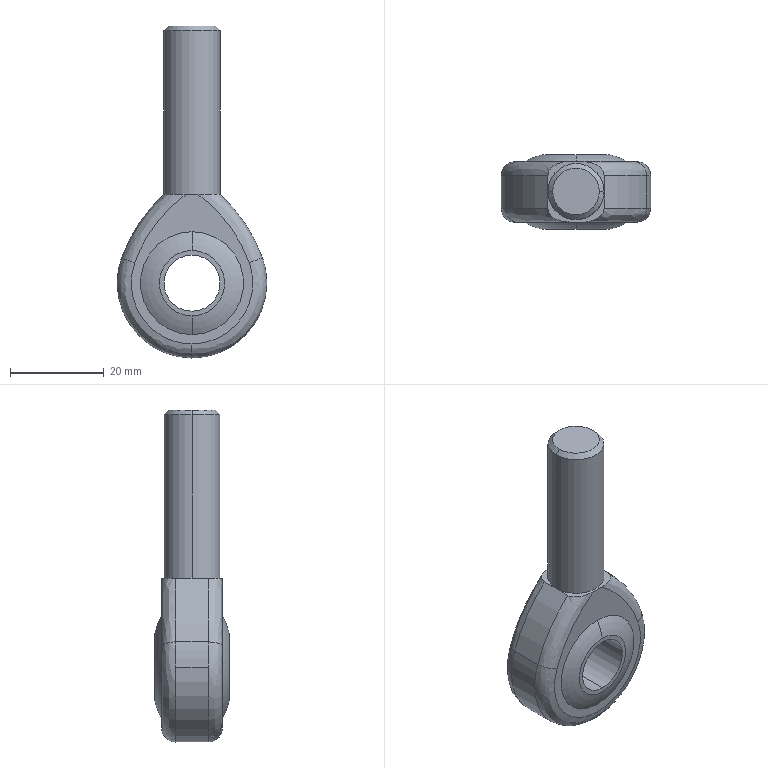Part | SolidWorks | features BaseBody 1 | 1 solid | 30 faces | box 32 x 16 x 71 mm | volume 14151 mm3 | cylinder 9 | spline 8 | plane 7 | torus 4 | cone 2 | commonest cylinder face diameters 12 x4 32 x3 67.817 x2
STEP:
#1=CARTESIAN_POINT('',(5.,0.,36.));
#2=VERTEX_POINT('',#1);
#3=CARTESIAN_POINT('',(-5.,0.,36.));
#4=VERTEX_POINT('',#3);
#5=CARTESIAN_POINT('',(0.,0.,36.));
#6=DIRECTION('',(0.,0.,1.));
#7=DIRECTION('',(-1.,0.,0.));
#8=AXIS2_PLACEMENT_3D('',#5,#6,#7);
#9=CIRCLE('',#8,5.);
#10=EDGE_CURVE('',#2,#4,#9,.T.);
#11=ORIENTED_EDGE('',*,*,#10,.F.);
#12=CARTESIAN_POINT('',(6.,0.,35.));
#13=VERTEX_POINT('',#12);
#14=CARTESIAN_POINT('',(5.,0.,36.));
#15=DIRECTION('',(0.7071,0.,-0.7071));
#16=VECTOR('',#15,1000.);
#17=LINE('',#14,#16);
#18=EDGE_CURVE('',#2,#13,#17,.T.);
#19=ORIENTED_EDGE('',*,*,#18,.T.);
#20=CARTESIAN_POINT('',(-6.,0.,35.));
#21=VERTEX_POINT('',#20);
#22=CARTESIAN_POINT('',(0.,0.,35.));
#23=DIRECTION('',(0.,0.,-1.));
#24=DIRECTION('',(-1.,0.,0.));
#25=AXIS2_PLACEMENT_3D('',#22,#23,#24);
#26=CIRCLE('',#25,6.);
#27=EDGE_CURVE('',#21,#13,#26,.T.);
#28=ORIENTED_EDGE('',*,*,#27,.F.);
#29=CARTESIAN_POINT('',(-5.,0.,36.));
#30=DIRECTION('',(-0.7071,0.,-0.7071));
#31=VECTOR('',#30,1000.);
#32=LINE('',#29,#31);
#33=EDGE_CURVE('',#4,#21,#32,.T.);
#34=ORIENTED_EDGE('',*,*,#33,.F.);
#35=EDGE_LOOP('',(#11,#19,#28,#34));
#36=FACE_OUTER_BOUND('',#35,.T.);
#37=CARTESIAN_POINT('',(0.,0.,36.));
#38=DIRECTION('',(0.,0.,-1.));
#39=DIRECTION('',(-1.,0.,0.));
#40=AXIS2_PLACEMENT_3D('',#37,#38,#39);
#41=CONICAL_SURFACE('',#40,5.,0.7854);
#42=ADVANCED_FACE('',(#36),#41,.T.);
#43=ORIENTED_EDGE('',*,*,#27,.T.);
#44=CARTESIAN_POINT('',(6.,0.,0.));
#45=VERTEX_POINT('',#44);
#46=CARTESIAN_POINT('',(6.,0.,35.));
#47=DIRECTION('',(0.,0.,-1.));
#48=VECTOR('',#47,1000.);
#49=LINE('',#46,#48);
#50=EDGE_CURVE('',#13,#45,#49,.T.);
#51=ORIENTED_EDGE('',*,*,#50,.T.);
#52=CARTESIAN_POINT('',(-6.,-0.000000001,0.));
#53=VERTEX_POINT('',#52);
#54=CARTESIAN_POINT('',(0.,0.,0.));
#55=DIRECTION('',(0.,0.,-1.));
#56=DIRECTION('',(-1.,0.,0.));
#57=AXIS2_PLACEMENT_3D('',#54,#55,#56);
#58=CIRCLE('',#57,6.);
#59=EDGE_CURVE('',#53,#45,#58,.T.);
#60=ORIENTED_EDGE('',*,*,#59,.F.);
#61=CARTESIAN_POINT('',(-6.,0.,35.));
#62=DIRECTION('',(0.,0.,-1.));
#63=VECTOR('',#62,1000.);
#64=LINE('',#61,#63);
#65=EDGE_CURVE('',#21,#53,#64,.T.);
#66=ORIENTED_EDGE('',*,*,#65,.F.);
#67=EDGE_LOOP('',(#43,#51,#60,#66));
#68=FACE_OUTER_BOUND('',#67,.T.);
#69=CARTESIAN_POINT('',(0.,0.,35.));
#70=DIRECTION('',(0.,0.,-1.));
#71=DIRECTION('',(-1.,0.,0.));
#72=AXIS2_PLACEMENT_3D('',#69,#70,#71);
#73=CYLINDRICAL_SURFACE('',#72,6.);
#74=ADVANCED_FACE('',(#68),#73,.T.);
#75=CARTESIAN_POINT('',(-16.,3.5,-19.));
#76=VERTEX_POINT('',#75);
#77=CARTESIAN_POINT('',(-15.06,3.5,-13.597));
#78=VERTEX_POINT('',#77);
#79=CARTESIAN_POINT('',(0.,3.5,-19.));
#80=DIRECTION('',(0.,1.,0.));
#81=DIRECTION('',(1.,0.,0.));
#82=AXIS2_PLACEMENT_3D('',#79,#80,#81);
#83=CIRCLE('',#82,16.);
#84=EDGE_CURVE('',#76,#78,#83,.T.);
#85=ORIENTED_EDGE('',*,*,#84,.F.);
#86=CARTESIAN_POINT('',(-16.,-3.5,-19.));
#87=VERTEX_POINT('',#86);
#88=CARTESIAN_POINT('',(-16.,3.5,-19.));
#89=DIRECTION('',(0.,-1.,0.));
#90=VECTOR('',#89,1000.);
#91=LINE('',#88,#90);
#92=EDGE_CURVE('',#76,#87,#91,.T.);
#93=ORIENTED_EDGE('',*,*,#92,.T.);
#94=CARTESIAN_POINT('',(-15.06,-3.5,-13.597));
#95=VERTEX_POINT('',#94);
#96=CARTESIAN_POINT('',(0.,-3.5,-19.));
#97=DIRECTION('',(0.,-1.,0.));
#98=DIRECTION('',(0.,0.,-1.));
#99=AXIS2_PLACEMENT_3D('',#96,#97,#98);
#100=CIRCLE('',#99,16.);
#101=EDGE_CURVE('',#95,#87,#100,.T.);
#102=ORIENTED_EDGE('',*,*,#101,.F.);
#103=CARTESIAN_POINT('',(-15.06,0.,-13.597));
#104=DIRECTION('',(0.,1.,0.));
#105=VECTOR('',#104,1000.);
#106=LINE('',#103,#105);
#107=EDGE_CURVE('',#95,#78,#106,.T.);
#108=ORIENTED_EDGE('',*,*,#107,.T.);
#109=EDGE_LOOP('',(#85,#93,#102,#108));
#110=FACE_OUTER_BOUND('',#109,.T.);
#111=CARTESIAN_POINT('',(0.,3.5,-19.));
#112=DIRECTION('',(0.,-1.,0.));
#113=DIRECTION('',(1.,0.,0.));
#114=AXIS2_PLACEMENT_3D('',#111,#112,#113);
#115=CYLINDRICAL_SURFACE('',#114,16.);
#116=ADVANCED_FACE('',(#110),#115,.T.);
#117=ORIENTED_EDGE('',*,*,#92,.F.);
#118=CARTESIAN_POINT('',(-0.000000001,3.5,-35.));
#119=VERTEX_POINT('',#118);
#120=CARTESIAN_POINT('',(0.,3.5,-19.));
#121=DIRECTION('',(0.,1.,0.));
#122=DIRECTION('',(1.,0.,0.));
#123=AXIS2_PLACEMENT_3D('',#120,#121,#122);
#124=CIRCLE('',#123,16.);
#125=EDGE_CURVE('',#119,#76,#124,.T.);
#126=ORIENTED_EDGE('',*,*,#125,.F.);
#127=CARTESIAN_POINT('',(16.,3.5,-19.));
#128=VERTEX_POINT('',#127);
#129=CARTESIAN_POINT('',(0.,3.5,-19.));
#130=DIRECTION('',(0.,1.,0.));
#131=DIRECTION('',(0.,0.,-1.));
#132=AXIS2_PLACEMENT_3D('',#129,#130,#131);
#133=CIRCLE('',#132,16.);
#134=EDGE_CURVE('',#128,#119,#133,.T.);
#135=ORIENTED_EDGE('',*,*,#134,.F.);
#136=CARTESIAN_POINT('',(16.,-3.5,-19.));
#137=VERTEX_POINT('',#136);
#138=CARTESIAN_POINT('',(16.,3.5,-19.));
#139=DIRECTION('',(0.,-1.,0.));
#140=VECTOR('',#139,1000.);
#141=LINE('',#138,#140);
#142=EDGE_CURVE('',#128,#137,#141,.T.);
#143=ORIENTED_EDGE('',*,*,#142,.T.);
#144=CARTESIAN_POINT('',(-0.000000001,-3.5,-35.));
#145=VERTEX_POINT('',#144);
#146=CARTESIAN_POINT('',(0.,-3.5,-19.));
#147=DIRECTION('',(0.,-1.,0.));
#148=DIRECTION('',(0.,0.,-1.));
#149=AXIS2_PLACEMENT_3D('',#146,#147,#148);
#150=CIRCLE('',#149,16.);
#151=EDGE_CURVE('',#145,#137,#150,.T.);
#152=ORIENTED_EDGE('',*,*,#151,.F.);
#153=CARTESIAN_POINT('',(0.,-3.5,-19.));
#154=DIRECTION('',(0.,-1.,0.));
#155=DIRECTION('',(0.,0.,-1.));
#156=AXIS2_PLACEMENT_3D('',#153,#154,#155);
#157=CIRCLE('',#156,16.);
#158=EDGE_CURVE('',#87,#145,#157,.T.);
#159=ORIENTED_EDGE('',*,*,#158,.F.);
#160=EDGE_LOOP('',(#117,#126,#135,#143,#152,#159));
#161=FACE_OUTER_BOUND('',#160,.T.);
#162=CARTESIAN_POINT('',(0.,3.5,-19.));
#163=DIRECTION('',(0.,-1.,0.));
#164=DIRECTION('',(1.,0.,0.));
#165=AXIS2_PLACEMENT_3D('',#162,#163,#164);
#166=CYLINDRICAL_SURFACE('',#165,16.);
#167=ADVANCED_FACE('',(#161),#166,.T.);
#168=CARTESIAN_POINT('',(0.,6.5,-7.994));
#169=VERTEX_POINT('',#168);
#170=CARTESIAN_POINT('',(0.,6.5,-30.006));
#171=VERTEX_POINT('',#170);
#172=CARTESIAN_POINT('',(0.,6.5,-19.));
#173=DIRECTION('',(0.,1.,0.));
#174=DIRECTION('',(0.,0.,1.));
#175=AXIS2_PLACEMENT_3D('',#172,#173,#174);
#176=CIRCLE('',#175,11.006);
#177=EDGE_CURVE('',#169,#171,#176,.T.);
#178=ORIENTED_EDGE('',*,*,#177,.T.);
#179=CARTESIAN_POINT('',(0.,8.,-26.));
#180=VERTEX_POINT('',#179);
#181=CARTESIAN_POINT('',(0.,-6.654,-22.797));
#182=DIRECTION('',(1.,0.,0.));
#183=DIRECTION('',(0.,0.,-1.));
#184=AXIS2_PLACEMENT_3D('',#181,#182,#183);
#185=CIRCLE('',#184,15.);
#186=EDGE_CURVE('',#171,#180,#185,.T.);
#187=ORIENTED_EDGE('',*,*,#186,.T.);
#188=CARTESIAN_POINT('',(0.,8.,-12.));
#189=VERTEX_POINT('',#188);
#190=CARTESIAN_POINT('',(0.,8.,-19.));
#191=DIRECTION('',(0.,-1.,0.));
#192=DIRECTION('',(0.,0.,1.));
#193=AXIS2_PLACEMENT_3D('',#190,#191,#192);
#194=CIRCLE('',#193,7.);
#195=EDGE_CURVE('',#180,#189,#194,.T.);
#196=ORIENTED_EDGE('',*,*,#195,.T.);
#197=CARTESIAN_POINT('',(0.,-6.654,-15.203));
#198=DIRECTION('',(-1.,0.,0.));
#199=DIRECTION('',(0.,0.,1.));
#200=AXIS2_PLACEMENT_3D('',#197,#198,#199);
#201=CIRCLE('',#200,15.);
#202=EDGE_CURVE('',#169,#189,#201,.T.);
#203=ORIENTED_EDGE('',*,*,#202,.F.);
#204=EDGE_LOOP('',(#178,#187,#196,#203));
#205=FACE_OUTER_BOUND('',#204,.T.);
#206=CARTESIAN_POINT('',(0.,-6.654,-19.));
#207=DIRECTION('',(0.,1.,0.));
#208=DIRECTION('',(0.,0.,1.));
#209=AXIS2_PLACEMENT_3D('',#206,#207,#208);
#210=TOROIDAL_SURFACE('',#209,3.797,15.);
#211=ADVANCED_FACE('',(#205),#210,.T.);
#212=CARTESIAN_POINT('',(0.,-6.5,-7.994));
#213=VERTEX_POINT('',#212);
#214=CARTESIAN_POINT('',(0.,-6.5,-30.006));
#215=VERTEX_POINT('',#214);
#216=CARTESIAN_POINT('',(0.,-6.5,-19.));
#217=DIRECTION('',(0.,1.,0.));
#218=DIRECTION('',(0.,0.,-1.));
#219=AXIS2_PLACEMENT_3D('',#216,#217,#218);
#220=CIRCLE('',#219,11.006);
#221=EDGE_CURVE('',#213,#215,#220,.T.);
#222=ORIENTED_EDGE('',*,*,#221,.F.);
#223=CARTESIAN_POINT('',(0.,-8.,-12.));
#224=VERTEX_POINT('',#223);
#225=CARTESIAN_POINT('',(0.,6.654,-15.203));
#226=DIRECTION('',(1.,0.,0.));
#227=DIRECTION('',(0.,0.,-1.));
#228=AXIS2_PLACEMENT_3D('',#225,#226,#227);
#229=CIRCLE('',#228,15.);
#230=EDGE_CURVE('',#213,#224,#229,.T.);
#231=ORIENTED_EDGE('',*,*,#230,.T.);
#232=CARTESIAN_POINT('',(0.,-8.,-26.));
#233=VERTEX_POINT('',#232);
#234=CARTESIAN_POINT('',(0.,-8.,-19.));
#235=DIRECTION('',(0.,1.,0.));
#236=DIRECTION('',(0.,0.,-1.));
#237=AXIS2_PLACEMENT_3D('',#234,#235,#236);
#238=CIRCLE('',#237,7.);
#239=EDGE_CURVE('',#224,#233,#238,.T.);
#240=ORIENTED_EDGE('',*,*,#239,.T.);
#241=CARTESIAN_POINT('',(0.,6.654,-22.797));
#242=DIRECTION('',(-1.,0.,0.));
#243=DIRECTION('',(0.,0.,1.));
#244=AXIS2_PLACEMENT_3D('',#241,#242,#243);
#245=CIRCLE('',#244,15.);
#246=EDGE_CURVE('',#215,#233,#245,.T.);
#247=ORIENTED_EDGE('',*,*,#246,.F.);
#248=EDGE_LOOP('',(#222,#231,#240,#247));
#249=FACE_OUTER_BOUND('',#248,.T.);
#250=CARTESIAN_POINT('',(0.,6.654,-19.));
#251=DIRECTION('',(0.,-1.,0.));
#252=DIRECTION('',(0.,0.,-1.));
#253=AXIS2_PLACEMENT_3D('',#250,#251,#252);
#254=TOROIDAL_SURFACE('',#253,3.797,15.);
#255=ADVANCED_FACE('',(#249),#254,.T.);
#256=CARTESIAN_POINT('',(0.,8.,-13.));
#257=VERTEX_POINT('',#256);
#258=CARTESIAN_POINT('',(0.,8.,-25.));
#259=VERTEX_POINT('',#258);
#260=CARTESIAN_POINT('',(0.,8.,-19.));
#261=DIRECTION('',(0.,-1.,0.));
#262=DIRECTION('',(0.,0.,-1.));
#263=AXIS2_PLACEMENT_3D('',#260,#261,#262);
#264=CIRCLE('',#263,6.);
#265=EDGE_CURVE('',#257,#259,#264,.T.);
#266=ORIENTED_EDGE('',*,*,#265,.F.);
#267=CARTESIAN_POINT('',(0.,-8.,-13.));
#268=VERTEX_POINT('',#267);
#269=CARTESIAN_POINT('',(0.,8.,-13.));
#270=DIRECTION('',(0.,-1.,0.));
#271=VECTOR('',#270,1000.);
#272=LINE('',#269,#271);
#273=EDGE_CURVE('',#257,#268,#272,.T.);
#274=ORIENTED_EDGE('',*,*,#273,.T.);
#275=CARTESIAN_POINT('',(0.,-8.,-25.));
#276=VERTEX_POINT('',#275);
#277=CARTESIAN_POINT('',(0.,-8.,-19.));
#278=DIRECTION('',(0.,1.,0.));
#279=DIRECTION('',(0.,0.,-1.));
#280=AXIS2_PLACEMENT_3D('',#277,#278,#279);
#281=CIRCLE('',#280,6.);
#282=EDGE_CURVE('',#276,#268,#281,.T.);
#283=ORIENTED_EDGE('',*,*,#282,.F.);
#284=CARTESIAN_POINT('',(0.,8.,-25.));
#285=DIRECTION('',(0.,-1.,0.));
#286=VECTOR('',#285,1000.);
#287=LINE('',#284,#286);
#288=EDGE_CURVE('',#259,#276,#287,.T.);
#289=ORIENTED_EDGE('',*,*,#288,.F.);
#290=EDGE_LOOP('',(#266,#274,#283,#289));
#291=FACE_OUTER_BOUND('',#290,.T.);
#292=CARTESIAN_POINT('',(0.,8.,-19.));
#293=DIRECTION('',(0.,-1.,0.));
#294=DIRECTION('',(0.,0.,-1.));
#295=AXIS2_PLACEMENT_3D('',#292,#293,#294);
#296=CYLINDRICAL_SURFACE('',#295,6.);
#297=ADVANCED_FACE('',(#291),#296,.F.);
#298=ORIENTED_EDGE('',*,*,#18,.F.);
#299=CARTESIAN_POINT('',(0.,0.,36.));
#300=DIRECTION('',(0.,0.,1.));
#301=DIRECTION('',(-1.,0.,0.));
#302=AXIS2_PLACEMENT_3D('',#299,#300,#301);
#303=CIRCLE('',#302,5.);
#304=EDGE_CURVE('',#4,#2,#303,.T.);
#305=ORIENTED_EDGE('',*,*,#304,.F.);
#306=ORIENTED_EDGE('',*,*,#33,.T.);
#307=CARTESIAN_POINT('',(0.,0.,35.));
#308=DIRECTION('',(0.,0.,-1.));
#309=DIRECTION('',(-1.,0.,0.));
#310=AXIS2_PLACEMENT_3D('',#307,#308,#309);
#311=CIRCLE('',#310,6.);
#312=EDGE_CURVE('',#13,#21,#311,.T.);
#313=ORIENTED_EDGE('',*,*,#312,.F.);
#314=EDGE_LOOP('',(#298,#305,#306,#313));
#315=FACE_OUTER_BOUND('',#314,.T.);
#316=CARTESIAN_POINT('',(0.,0.,36.));
#317=DIRECTION('',(0.,0.,-1.));
#318=DIRECTION('',(-1.,0.,0.));
#319=AXIS2_PLACEMENT_3D('',#316,#317,#318);
#320=CONICAL_SURFACE('',#319,5.,0.7854);
#321=ADVANCED_FACE('',(#315),#320,.T.);
#322=ORIENTED_EDGE('',*,*,#304,.T.);
#323=ORIENTED_EDGE('',*,*,#10,.T.);
#324=EDGE_LOOP('',(#322,#323));
#325=FACE_OUTER_BOUND('',#324,.T.);
#326=CARTESIAN_POINT('',(-5.06,-5.06,36.));
#327=DIRECTION('',(0.,0.,1.));
#328=DIRECTION('',(1.,0.,0.));
#329=AXIS2_PLACEMENT_3D('',#326,#327,#328);
#330=PLANE('',#329);
#331=ADVANCED_FACE('',(#325),#330,.T.);
#332=ORIENTED_EDGE('',*,*,#50,.F.);
#333=ORIENTED_EDGE('',*,*,#312,.T.);
#334=ORIENTED_EDGE('',*,*,#65,.T.);
#335=CARTESIAN_POINT('',(0.,0.,0.));
#336=DIRECTION('',(0.,0.,-1.));
#337=DIRECTION('',(-1.,0.,0.));
#338=AXIS2_PLACEMENT_3D('',#335,#336,#337);
#339=CIRCLE('',#338,6.);
#340=EDGE_CURVE('',#45,#53,#339,.T.);
#341=ORIENTED_EDGE('',*,*,#340,.F.);
#342=EDGE_LOOP('',(#332,#333,#334,#341));
#343=FACE_OUTER_BOUND('',#342,.T.);
#344=CARTESIAN_POINT('',(0.,0.,35.));
#345=DIRECTION('',(0.,0.,-1.));
#346=DIRECTION('',(-1.,0.,0.));
#347=AXIS2_PLACEMENT_3D('',#344,#345,#346);
#348=CYLINDRICAL_SURFACE('',#347,6.);
#349=ADVANCED_FACE('',(#343),#348,.T.);
#350=CARTESIAN_POINT('',(1.253,6.5,0.));
#351=VERTEX_POINT('',#350);
#352=CARTESIAN_POINT('',(6.,3.5,0.));
#353=VERTEX_POINT('',#352);
#354=CARTESIAN_POINT('',(1.253,6.5,0.));
#355=CARTESIAN_POINT('',(1.771,6.5,0.));
#356=CARTESIAN_POINT('',(2.28,6.455,0.));
#357=CARTESIAN_POINT('',(3.029,6.306,0.));
#358=CARTESIAN_POINT('',(3.277,6.243,0.));
#359=CARTESIAN_POINT('',(3.766,6.083,0.));
#360=CARTESIAN_POINT('',(4.008,5.986,0.));
#361=CARTESIAN_POINT('',(4.471,5.755,0.));
#362=CARTESIAN_POINT('',(4.691,5.621,0.));
#363=CARTESIAN_POINT('',(5.107,5.306,0.));
#364=CARTESIAN_POINT('',(5.295,5.13,0.));
#365=CARTESIAN_POINT('',(5.54,4.829,0.));
#366=CARTESIAN_POINT('',(5.616,4.722,0.));
#367=CARTESIAN_POINT('',(5.749,4.499,0.));
#368=CARTESIAN_POINT('',(5.806,4.383,0.));
#369=CARTESIAN_POINT('',(5.901,4.142,0.));
#370=CARTESIAN_POINT('',(5.938,4.016,0.));
#371=CARTESIAN_POINT('',(5.987,3.76,0.));
#372=CARTESIAN_POINT('',(6.,3.631,0.));
#373=CARTESIAN_POINT('',(6.,3.5,0.));
#374=B_SPLINE_CURVE_WITH_KNOTS('',3,(#354,#355,#356,#357,#358,#359,#360,#361,#362,#363,#364,#365,#366,#367,#368,#369,#370,#371,#372,#373),.UNSPECIFIED.,.F.,.F.,(4,2,2,2,2,2,2,2,2,4),(0.,0.001528,0.002292,0.003056,0.00382,0.004584,0.004965,0.005347,0.005729,0.006111),.UNSPECIFIED.);
#375=EDGE_CURVE('',#351,#353,#374,.T.);
#376=ORIENTED_EDGE('',*,*,#375,.F.);
#377=CARTESIAN_POINT('',(-1.253,6.5,0.));
#378=VERTEX_POINT('',#377);
#379=CARTESIAN_POINT('',(0.,6.5,0.));
#380=DIRECTION('',(1.,0.,0.));
#381=VECTOR('',#380,1000.);
#382=LINE('',#379,#381);
#383=EDGE_CURVE('',#378,#351,#382,.T.);
#384=ORIENTED_EDGE('',*,*,#383,.F.);
#385=CARTESIAN_POINT('',(-6.,3.5,0.));
#386=VERTEX_POINT('',#385);
#387=CARTESIAN_POINT('',(-6.,3.5,0.));
#388=CARTESIAN_POINT('',(-6.,3.762,0.));
#389=CARTESIAN_POINT('',(-5.95,4.014,0.));
#390=CARTESIAN_POINT('',(-5.761,4.501,0.));
#391=CARTESIAN_POINT('',(-5.627,4.722,0.));
#392=CARTESIAN_POINT('',(-5.298,5.127,0.));
#393=CARTESIAN_POINT('',(-5.111,5.303,0.));
#394=CARTESIAN_POINT('',(-4.701,5.615,0.));
#395=CARTESIAN_POINT('',(-4.477,5.751,0.));
#396=CARTESIAN_POINT('',(-4.018,5.981,0.));
#397=CARTESIAN_POINT('',(-3.78,6.078,0.));
#398=CARTESIAN_POINT('',(-3.292,6.239,0.));
#399=CARTESIAN_POINT('',(-3.04,6.304,0.));
#400=CARTESIAN_POINT('',(-2.283,6.455,0.));
#401=CARTESIAN_POINT('',(-1.771,6.5,0.));
#402=CARTESIAN_POINT('',(-1.253,6.5,0.));
#403=B_SPLINE_CURVE_WITH_KNOTS('',3,(#387,#388,#389,#390,#391,#392,#393,#394,#395,#396,#397,#398,#399,#400,#401,#402),.UNSPECIFIED.,.F.,.F.,(4,2,2,2,2,2,2,4),(0.,0.0007712,0.001542,0.002314,0.003085,0.003856,0.004627,0.006169),.UNSPECIFIED.);
#404=EDGE_CURVE('',#386,#378,#403,.T.);
#405=ORIENTED_EDGE('',*,*,#404,.F.);
#406=CARTESIAN_POINT('',(-6.,3.231,0.));
#407=DIRECTION('',(0.,1.,0.));
#408=VECTOR('',#407,1000.);
#409=LINE('',#406,#408);
#410=EDGE_CURVE('',#53,#386,#409,.T.);
#411=ORIENTED_EDGE('',*,*,#410,.F.);
#412=ORIENTED_EDGE('',*,*,#59,.T.);
#413=CARTESIAN_POINT('',(6.,3.231,0.));
#414=DIRECTION('',(0.,-1.,0.));
#415=VECTOR('',#414,1000.);
#416=LINE('',#413,#415);
#417=EDGE_CURVE('',#353,#45,#416,.T.);
#418=ORIENTED_EDGE('',*,*,#417,.F.);
#419=EDGE_LOOP('',(#376,#384,#405,#411,#412,#418));
#420=FACE_OUTER_BOUND('',#419,.T.);
#421=CARTESIAN_POINT('',(6.,-0.039,0.));
#422=DIRECTION('',(0.,0.,-1.));
#423=DIRECTION('',(-1.,0.,0.));
#424=AXIS2_PLACEMENT_3D('',#421,#422,#423);
#425=PLANE('',#424);
#426=ADVANCED_FACE('',(#420),#425,.F.);
#427=CARTESIAN_POINT('',(6.,-3.5,0.));
#428=VERTEX_POINT('',#427);
#429=CARTESIAN_POINT('',(1.253,-6.5,0.));
#430=VERTEX_POINT('',#429);
#431=CARTESIAN_POINT('',(6.,-3.5,0.));
#432=CARTESIAN_POINT('',(6.,-3.762,0.));
#433=CARTESIAN_POINT('',(5.95,-4.014,0.));
#434=CARTESIAN_POINT('',(5.761,-4.501,0.));
#435=CARTESIAN_POINT('',(5.627,-4.722,0.));
#436=CARTESIAN_POINT('',(5.298,-5.127,0.));
#437=CARTESIAN_POINT('',(5.111,-5.303,0.));
#438=CARTESIAN_POINT('',(4.701,-5.615,0.));
#439=CARTESIAN_POINT('',(4.477,-5.751,0.));
#440=CARTESIAN_POINT('',(4.018,-5.981,0.));
#441=CARTESIAN_POINT('',(3.78,-6.078,0.));
#442=CARTESIAN_POINT('',(3.292,-6.239,0.));
#443=CARTESIAN_POINT('',(3.04,-6.304,0.));
#444=CARTESIAN_POINT('',(2.283,-6.455,0.));
#445=CARTESIAN_POINT('',(1.771,-6.5,0.));
#446=CARTESIAN_POINT('',(1.253,-6.5,0.));
#447=B_SPLINE_CURVE_WITH_KNOTS('',3,(#431,#432,#433,#434,#435,#436,#437,#438,#439,#440,#441,#442,#443,#444,#445,#446),.UNSPECIFIED.,.F.,.F.,(4,2,2,2,2,2,2,4),(0.,0.0007712,0.001542,0.002314,0.003085,0.003856,0.004627,0.006169),.UNSPECIFIED.);
#448=EDGE_CURVE('',#428,#430,#447,.T.);
#449=ORIENTED_EDGE('',*,*,#448,.F.);
#450=CARTESIAN_POINT('',(6.,-3.231,0.));
#451=DIRECTION('',(0.,-1.,0.));
#452=VECTOR('',#451,1000.);
#453=LINE('',#450,#452);
#454=EDGE_CURVE('',#45,#428,#453,.T.);
#455=ORIENTED_EDGE('',*,*,#454,.F.);
#456=ORIENTED_EDGE('',*,*,#340,.T.);
#457=CARTESIAN_POINT('',(-6.,-3.5,0.));
#458=VERTEX_POINT('',#457);
#459=CARTESIAN_POINT('',(-6.,-3.231,0.));
#460=DIRECTION('',(0.,1.,0.));
#461=VECTOR('',#460,1000.);
#462=LINE('',#459,#461);
#463=EDGE_CURVE('',#458,#53,#462,.T.);
#464=ORIENTED_EDGE('',*,*,#463,.F.);
#465=CARTESIAN_POINT('',(-1.253,-6.5,0.));
#466=VERTEX_POINT('',#465);
#467=CARTESIAN_POINT('',(-1.253,-6.5,0.));
#468=CARTESIAN_POINT('',(-1.771,-6.5,0.));
#469=CARTESIAN_POINT('',(-2.28,-6.455,0.));
#470=CARTESIAN_POINT('',(-3.029,-6.306,0.));
#471=CARTESIAN_POINT('',(-3.277,-6.243,0.));
#472=CARTESIAN_POINT('',(-3.766,-6.083,0.));
#473=CARTESIAN_POINT('',(-4.008,-5.986,0.));
#474=CARTESIAN_POINT('',(-4.471,-5.755,0.));
#475=CARTESIAN_POINT('',(-4.691,-5.621,0.));
#476=CARTESIAN_POINT('',(-5.107,-5.306,0.));
#477=CARTESIAN_POINT('',(-5.295,-5.13,0.));
#478=CARTESIAN_POINT('',(-5.54,-4.829,0.));
#479=CARTESIAN_POINT('',(-5.616,-4.722,0.));
#480=CARTESIAN_POINT('',(-5.749,-4.499,0.));
#481=CARTESIAN_POINT('',(-5.806,-4.383,0.));
#482=CARTESIAN_POINT('',(-5.901,-4.142,0.));
#483=CARTESIAN_POINT('',(-5.938,-4.016,0.));
#484=CARTESIAN_POINT('',(-5.987,-3.76,0.));
#485=CARTESIAN_POINT('',(-6.,-3.631,0.));
#486=CARTESIAN_POINT('',(-6.,-3.5,0.));
#487=B_SPLINE_CURVE_WITH_KNOTS('',3,(#467,#468,#469,#470,#471,#472,#473,#474,#475,#476,#477,#478,#479,#480,#481,#482,#483,#484,#485,#486),.UNSPECIFIED.,.F.,.F.,(4,2,2,2,2,2,2,2,2,4),(0.,0.001528,0.002292,0.003056,0.00382,0.004584,0.004965,0.005347,0.005729,0.006111),.UNSPECIFIED.);
#488=EDGE_CURVE('',#466,#458,#487,.T.);
#489=ORIENTED_EDGE('',*,*,#488,.F.);
#490=CARTESIAN_POINT('',(0.,-6.5,0.));
#491=DIRECTION('',(-1.,0.,0.));
#492=VECTOR('',#491,1000.);
#493=LINE('',#490,#492);
#494=EDGE_CURVE('',#430,#466,#493,.T.);
#495=ORIENTED_EDGE('',*,*,#494,.F.);
#496=EDGE_LOOP('',(#449,#455,#456,#464,#489,#495));
#497=FACE_OUTER_BOUND('',#496,.T.);
#498=CARTESIAN_POINT('',(6.,-6.5,0.));
#499=DIRECTION('',(0.,0.,-1.));
#500=DIRECTION('',(-1.,0.,0.));
#501=AXIS2_PLACEMENT_3D('',#498,#499,#500);
#502=PLANE('',#501);
#503=ADVANCED_FACE('',(#497),#502,.F.);
#504=CARTESIAN_POINT('',(15.06,-3.5,-13.597));
#505=VERTEX_POINT('',#504);
#506=CARTESIAN_POINT('',(-16.857,-3.5,-25.047));
#507=DIRECTION('',(0.,-1.,0.));
#508=DIRECTION('',(0.,0.,-1.));
#509=AXIS2_PLACEMENT_3D('',#506,#507,#508);
#510=CIRCLE('',#509,33.908);
#511=EDGE_CURVE('',#505,#428,#510,.T.);
#512=ORIENTED_EDGE('',*,*,#511,.F.);
#513=CARTESIAN_POINT('',(15.06,3.5,-13.597));
#514=VERTEX_POINT('',#513);
#515=CARTESIAN_POINT('',(15.06,0.,-13.597));
#516=DIRECTION('',(0.,-1.,0.));
#517=VECTOR('',#516,1000.);
#518=LINE('',#515,#517);
#519=EDGE_CURVE('',#514,#505,#518,.T.);
#520=ORIENTED_EDGE('',*,*,#519,.F.);
#521=CARTESIAN_POINT('',(-16.857,3.5,-25.047));
#522=DIRECTION('',(0.,1.,0.));
#523=DIRECTION('',(0.,0.,-1.));
#524=AXIS2_PLACEMENT_3D('',#521,#522,#523);
#525=CIRCLE('',#524,33.908);
#526=EDGE_CURVE('',#353,#514,#525,.T.);
#527=ORIENTED_EDGE('',*,*,#526,.F.);
#528=ORIENTED_EDGE('',*,*,#417,.T.);
#529=ORIENTED_EDGE('',*,*,#454,.T.);
#530=EDGE_LOOP('',(#512,#520,#527,#528,#529));
#531=FACE_OUTER_BOUND('',#530,.T.);
#532=CARTESIAN_POINT('',(-16.857,3.5,-25.047));
#533=DIRECTION('',(0.,-1.,0.));
#534=DIRECTION('',(1.,0.,0.));
#535=AXIS2_PLACEMENT_3D('',#532,#533,#534);
#536=CYLINDRICAL_SURFACE('',#535,33.908);
#537=ADVANCED_FACE('',(#531),#536,.T.);
#538=CARTESIAN_POINT('',(12.236,6.5,-14.61));
#539=VERTEX_POINT('',#538);
#540=CARTESIAN_POINT('',(15.06,3.5,-13.597));
#541=CARTESIAN_POINT('',(15.06,5.257,-13.597));
#542=CARTESIAN_POINT('',(13.891,6.5,-14.017));
#543=CARTESIAN_POINT('',(12.236,6.5,-14.61));
#544=(BOUNDED_CURVE()B_SPLINE_CURVE(3,(#540,#541,#542,#543),.UNSPECIFIED.,.F.,.F.)B_SPLINE_CURVE_WITH_KNOTS((4,4),(0.06314,0.9369),.UNSPECIFIED.)CURVE()GEOMETRIC_REPRESENTATION_ITEM()RATIONAL_B_SPLINE_CURVE((0.9566,0.7698,0.7698,0.9566))REPRESENTATION_ITEM(''));
#545=EDGE_CURVE('',#514,#539,#544,.T.);
#546=ORIENTED_EDGE('',*,*,#545,.T.);
#547=CARTESIAN_POINT('',(12.236,6.5,-14.61));
#548=CARTESIAN_POINT('',(10.116,6.5,-8.7));
#549=CARTESIAN_POINT('',(6.343,6.5,-3.68));
#550=CARTESIAN_POINT('',(1.253,6.5,0.));
#551=(BOUNDED_CURVE()B_SPLINE_CURVE(3,(#547,#548,#549,#550),.UNSPECIFIED.,.F.,.T.)B_SPLINE_CURVE_WITH_KNOTS((4,4),(0.,1.),.UNSPECIFIED.)CURVE()GEOMETRIC_REPRESENTATION_ITEM()RATIONAL_B_SPLINE_CURVE((0.9566,0.9279,0.9277,0.9561))REPRESENTATION_ITEM(''));
#552=EDGE_CURVE('',#539,#351,#551,.T.);
#553=ORIENTED_EDGE('',*,*,#552,.T.);
#554=ORIENTED_EDGE('',*,*,#375,.T.);
#555=ORIENTED_EDGE('',*,*,#526,.T.);
#556=EDGE_LOOP('',(#546,#553,#554,#555));
#557=FACE_OUTER_BOUND('',#556,.T.);
#558=CARTESIAN_POINT('',(15.046,3.2,-13.602));
#559=CARTESIAN_POINT('',(12.706,3.2,-7.08));
#560=CARTESIAN_POINT('',(8.533,3.2,-1.549));
#561=CARTESIAN_POINT('',(2.903,3.2,2.49));
#562=CARTESIAN_POINT('',(15.239,5.24,-13.533));
#563=CARTESIAN_POINT('',(12.885,5.24,-6.972));
#564=CARTESIAN_POINT('',(8.686,5.24,-1.407));
#565=CARTESIAN_POINT('',(3.023,5.24,2.657));
#566=CARTESIAN_POINT('',(13.874,6.69,-14.023));
#567=CARTESIAN_POINT('',(11.621,6.69,-7.74));
#568=CARTESIAN_POINT('',(7.6,6.69,-2.412));
#569=CARTESIAN_POINT('',(2.178,6.69,1.479));
#570=CARTESIAN_POINT('',(11.955,6.485,-14.711));
#571=CARTESIAN_POINT('',(9.842,6.485,-8.821));
#572=CARTESIAN_POINT('',(6.073,6.485,-3.826));
#573=CARTESIAN_POINT('',(0.9885,6.485,-0.1783));
#574=(BOUNDED_SURFACE()B_SPLINE_SURFACE(3,3,((#558,#559,#560,#561),(#562,#563,#564,#565),(#566,#567,#568,#569),(#570,#571,#572,#573)),.UNSPECIFIED.,.F.,.F.,.T.)B_SPLINE_SURFACE_WITH_KNOTS((4,4),(4,4),(0.,1.),(0.,1.),.UNSPECIFIED.)GEOMETRIC_REPRESENTATION_ITEM()RATIONAL_B_SPLINE_SURFACE(((1.,0.9698,0.9698,1.),(0.7553,0.7325,0.7325,0.7553),(0.7553,0.7325,0.7325,0.7553),(1.,0.9698,0.9698,1.)))REPRESENTATION_ITEM('')SURFACE());
#575=ADVANCED_FACE('',(#557),#574,.T.);
#576=ORIENTED_EDGE('',*,*,#177,.F.);
#577=CARTESIAN_POINT('',(0.,6.5,-19.));
#578=DIRECTION('',(0.,1.,0.));
#579=DIRECTION('',(0.,0.,1.));
#580=AXIS2_PLACEMENT_3D('',#577,#578,#579);
#581=CIRCLE('',#580,11.006);
#582=EDGE_CURVE('',#171,#169,#581,.T.);
#583=ORIENTED_EDGE('',*,*,#582,.F.);
#584=EDGE_LOOP('',(#576,#583));
#585=FACE_BOUND('',#584,.T.);
#586=ORIENTED_EDGE('',*,*,#552,.F.);
#587=CARTESIAN_POINT('',(0.,6.5,-32.));
#588=VERTEX_POINT('',#587);
#589=CARTESIAN_POINT('',(0.,6.5,-32.));
#590=CARTESIAN_POINT('',(9.886,6.5,-32.));
#591=CARTESIAN_POINT('',(15.575,6.5,-23.915));
#592=CARTESIAN_POINT('',(12.236,6.5,-14.61));
#593=(BOUNDED_CURVE()B_SPLINE_CURVE(3,(#589,#590,#591,#592),.UNSPECIFIED.,.F.,.F.)B_SPLINE_CURVE_WITH_KNOTS((4,4),(0.,1.),.UNSPECIFIED.)CURVE()GEOMETRIC_REPRESENTATION_ITEM()RATIONAL_B_SPLINE_CURVE((0.9566,0.6858,0.6858,0.9566))REPRESENTATION_ITEM(''));
#594=EDGE_CURVE('',#588,#539,#593,.T.);
#595=ORIENTED_EDGE('',*,*,#594,.F.);
#596=CARTESIAN_POINT('',(-12.236,6.5,-14.61));
#597=VERTEX_POINT('',#596);
#598=CARTESIAN_POINT('',(-12.236,6.5,-14.61));
#599=CARTESIAN_POINT('',(-15.575,6.5,-23.915));
#600=CARTESIAN_POINT('',(-9.886,6.5,-32.));
#601=CARTESIAN_POINT('',(0.,6.5,-32.));
#602=(BOUNDED_CURVE()B_SPLINE_CURVE(3,(#598,#599,#600,#601),.UNSPECIFIED.,.F.,.F.)B_SPLINE_CURVE_WITH_KNOTS((4,4),(0.,1.),.UNSPECIFIED.)CURVE()GEOMETRIC_REPRESENTATION_ITEM()RATIONAL_B_SPLINE_CURVE((0.9566,0.6858,0.6858,0.9566))REPRESENTATION_ITEM(''));
#603=EDGE_CURVE('',#597,#588,#602,.T.);
#604=ORIENTED_EDGE('',*,*,#603,.F.);
#605=CARTESIAN_POINT('',(-1.253,6.5,0.));
#606=CARTESIAN_POINT('',(-6.343,6.5,-3.68));
#607=CARTESIAN_POINT('',(-10.116,6.5,-8.7));
#608=CARTESIAN_POINT('',(-12.236,6.5,-14.61));
#609=(BOUNDED_CURVE()B_SPLINE_CURVE(3,(#605,#606,#607,#608),.UNSPECIFIED.,.F.,.F.)B_SPLINE_CURVE_WITH_KNOTS((4,4),(0.,1.),.UNSPECIFIED.)CURVE()GEOMETRIC_REPRESENTATION_ITEM()RATIONAL_B_SPLINE_CURVE((0.9561,0.9277,0.9279,0.9566))REPRESENTATION_ITEM(''));
#610=EDGE_CURVE('',#378,#597,#609,.T.);
#611=ORIENTED_EDGE('',*,*,#610,.F.);
#612=ORIENTED_EDGE('',*,*,#383,.T.);
#613=EDGE_LOOP('',(#586,#595,#604,#611,#612));
#614=FACE_OUTER_BOUND('',#613,.T.);
#615=CARTESIAN_POINT('',(-13.156,6.5,0.));
#616=DIRECTION('',(0.,-1.,0.));
#617=DIRECTION('',(0.,0.,-1.));
#618=AXIS2_PLACEMENT_3D('',#615,#616,#617);
#619=PLANE('',#618);
#620=ADVANCED_FACE('',(#585,#614),#619,.F.);
#621=CARTESIAN_POINT('',(-12.236,6.5,-14.61));
#622=CARTESIAN_POINT('',(-13.891,6.5,-14.017));
#623=CARTESIAN_POINT('',(-15.06,5.257,-13.597));
#624=CARTESIAN_POINT('',(-15.06,3.5,-13.597));
#625=(BOUNDED_CURVE()B_SPLINE_CURVE(3,(#621,#622,#623,#624),.UNSPECIFIED.,.F.,.T.)B_SPLINE_CURVE_WITH_KNOTS((4,4),(0.06314,0.9369),.UNSPECIFIED.)CURVE()GEOMETRIC_REPRESENTATION_ITEM()RATIONAL_B_SPLINE_CURVE((0.9566,0.7698,0.7698,0.9566))REPRESENTATION_ITEM(''));
#626=EDGE_CURVE('',#597,#78,#625,.T.);
#627=ORIENTED_EDGE('',*,*,#626,.T.);
#628=CARTESIAN_POINT('',(16.857,3.5,-25.047));
#629=DIRECTION('',(0.,1.,0.));
#630=DIRECTION('',(1.,0.,0.));
#631=AXIS2_PLACEMENT_3D('',#628,#629,#630);
#632=CIRCLE('',#631,33.908);
#633=EDGE_CURVE('',#78,#386,#632,.T.);
#634=ORIENTED_EDGE('',*,*,#633,.T.);
#635=ORIENTED_EDGE('',*,*,#404,.T.);
#636=ORIENTED_EDGE('',*,*,#610,.T.);
#637=EDGE_LOOP('',(#627,#634,#635,#636));
#638=FACE_OUTER_BOUND('',#637,.T.);
#639=CARTESIAN_POINT('',(-2.903,3.2,2.49));
#640=CARTESIAN_POINT('',(-8.533,3.2,-1.549));
#641=CARTESIAN_POINT('',(-12.706,3.2,-7.08));
#642=CARTESIAN_POINT('',(-15.046,3.2,-13.602));
#643=CARTESIAN_POINT('',(-3.023,5.24,2.657));
#644=CARTESIAN_POINT('',(-8.686,5.24,-1.407));
#645=CARTESIAN_POINT('',(-12.885,5.24,-6.972));
#646=CARTESIAN_POINT('',(-15.239,5.24,-13.533));
#647=CARTESIAN_POINT('',(-2.178,6.69,1.479));
#648=CARTESIAN_POINT('',(-7.6,6.69,-2.412));
#649=CARTESIAN_POINT('',(-11.621,6.69,-7.74));
#650=CARTESIAN_POINT('',(-13.874,6.69,-14.023));
#651=CARTESIAN_POINT('',(-0.9885,6.485,-0.1783));
#652=CARTESIAN_POINT('',(-6.073,6.485,-3.826));
#653=CARTESIAN_POINT('',(-9.842,6.485,-8.821));
#654=CARTESIAN_POINT('',(-11.955,6.485,-14.711));
#655=(BOUNDED_SURFACE()B_SPLINE_SURFACE(3,3,((#639,#640,#641,#642),(#643,#644,#645,#646),(#647,#648,#649,#650),(#651,#652,#653,#654)),.UNSPECIFIED.,.F.,.F.,.T.)B_SPLINE_SURFACE_WITH_KNOTS((4,4),(4,4),(0.,1.),(0.,1.),.UNSPECIFIED.)GEOMETRIC_REPRESENTATION_ITEM()RATIONAL_B_SPLINE_SURFACE(((1.,0.9698,0.9698,1.),(0.7553,0.7325,0.7325,0.7553),(0.7553,0.7325,0.7325,0.7553),(1.,0.9698,0.9698,1.)))REPRESENTATION_ITEM('')SURFACE());
#656=ADVANCED_FACE('',(#638),#655,.T.);
#657=CARTESIAN_POINT('',(16.857,-3.5,-25.047));
#658=DIRECTION('',(0.,-1.,0.));
#659=DIRECTION('',(0.,0.,-1.));
#660=AXIS2_PLACEMENT_3D('',#657,#658,#659);
#661=CIRCLE('',#660,33.908);
#662=EDGE_CURVE('',#458,#95,#661,.T.);
#663=ORIENTED_EDGE('',*,*,#662,.F.);
#664=ORIENTED_EDGE('',*,*,#463,.T.);
#665=ORIENTED_EDGE('',*,*,#410,.T.);
#666=ORIENTED_EDGE('',*,*,#633,.F.);
#667=ORIENTED_EDGE('',*,*,#107,.F.);
#668=EDGE_LOOP('',(#663,#664,#665,#666,#667));
#669=FACE_OUTER_BOUND('',#668,.T.);
#670=CARTESIAN_POINT('',(16.857,3.5,-25.047));
#671=DIRECTION('',(0.,-1.,0.));
#672=DIRECTION('',(1.,0.,0.));
#673=AXIS2_PLACEMENT_3D('',#670,#671,#672);
#674=CYLINDRICAL_SURFACE('',#673,33.908);
#675=ADVANCED_FACE('',(#669),#674,.T.);
#676=CARTESIAN_POINT('',(0.,-6.5,-19.));
#677=DIRECTION('',(0.,1.,0.));
#678=DIRECTION('',(0.,0.,-1.));
#679=AXIS2_PLACEMENT_3D('',#676,#677,#678);
#680=CIRCLE('',#679,11.006);
#681=EDGE_CURVE('',#215,#213,#680,.T.);
#682=ORIENTED_EDGE('',*,*,#681,.T.);
#683=ORIENTED_EDGE('',*,*,#221,.T.);
#684=EDGE_LOOP('',(#682,#683));
#685=FACE_BOUND('',#684,.T.);
#686=ORIENTED_EDGE('',*,*,#494,.T.);
#687=CARTESIAN_POINT('',(-12.236,-6.5,-14.61));
#688=VERTEX_POINT('',#687);
#689=CARTESIAN_POINT('',(-1.253,-6.5,0.));
#690=CARTESIAN_POINT('',(-1.878,-6.5,-0.4513));
#691=CARTESIAN_POINT('',(-2.786,-6.5,-1.161));
#692=CARTESIAN_POINT('',(-3.798,-6.5,-2.047));
#693=CARTESIAN_POINT('',(-4.221,-6.5,-2.439));
#694=CARTESIAN_POINT('',(-4.501,-6.5,-2.703));
#695=CARTESIAN_POINT('',(-4.638,-6.5,-2.835));
#696=CARTESIAN_POINT('',(-5.889,-6.5,-4.062));
#697=CARTESIAN_POINT('',(-6.915,-6.5,-5.231));
#698=CARTESIAN_POINT('',(-8.318,-6.5,-7.098));
#699=CARTESIAN_POINT('',(-8.983,-6.5,-8.056));
#700=CARTESIAN_POINT('',(-9.694,-6.5,-9.215));
#701=CARTESIAN_POINT('',(-10.033,-6.5,-9.805));
#702=CARTESIAN_POINT('',(-10.175,-6.5,-10.06));
#703=CARTESIAN_POINT('',(-10.269,-6.5,-10.23));
#704=CARTESIAN_POINT('',(-10.316,-6.5,-10.317));
#705=CARTESIAN_POINT('',(-11.091,-6.5,-11.758));
#706=CARTESIAN_POINT('',(-11.716,-6.5,-13.161));
#707=CARTESIAN_POINT('',(-12.236,-6.5,-14.61));
#708=B_SPLINE_CURVE_WITH_KNOTS('',3,(#689,#690,#691,#692,#693,#694,#695,#696,#697,#698,#699,#700,#701,#702,#703,#704,#705,#706,#707),.UNSPECIFIED.,.F.,.F.,(4,1,1,2,2,2,1,1,1,2,2,4),(0.,0.125,0.1875,0.2188,0.25,0.5,0.625,0.6875,0.7188,0.7344,0.75,1.),.UNSPECIFIED.);
#709=EDGE_CURVE('',#466,#688,#708,.T.);
#710=ORIENTED_EDGE('',*,*,#709,.T.);
#711=CARTESIAN_POINT('',(0.,-6.5,-32.));
#712=VERTEX_POINT('',#711);
#713=CARTESIAN_POINT('',(-12.236,-6.5,-14.61));
#714=CARTESIAN_POINT('',(-12.313,-6.5,-14.824));
#715=CARTESIAN_POINT('',(-12.42,-6.5,-15.148));
#716=CARTESIAN_POINT('',(-12.529,-6.5,-15.53));
#717=CARTESIAN_POINT('',(-12.58,-6.5,-15.723));
#718=CARTESIAN_POINT('',(-12.601,-6.5,-15.805));
#719=CARTESIAN_POINT('',(-12.615,-6.5,-15.861));
#720=CARTESIAN_POINT('',(-12.622,-6.5,-15.887));
#721=CARTESIAN_POINT('',(-12.686,-6.5,-16.148));
#722=CARTESIAN_POINT('',(-12.761,-6.5,-16.498));
#723=CARTESIAN_POINT('',(-12.832,-6.5,-16.909));
#724=CARTESIAN_POINT('',(-12.863,-6.5,-17.116));
#725=CARTESIAN_POINT('',(-12.875,-6.5,-17.205));
#726=CARTESIAN_POINT('',(-12.884,-6.5,-17.264));
#727=CARTESIAN_POINT('',(-12.887,-6.5,-17.292));
#728=CARTESIAN_POINT('',(-12.924,-6.5,-17.57));
#729=CARTESIAN_POINT('',(-12.961,-6.5,-17.942));
#730=CARTESIAN_POINT('',(-12.986,-6.5,-18.378));
#731=CARTESIAN_POINT('',(-12.994,-6.5,-18.596));
#732=CARTESIAN_POINT('',(-12.996,-6.5,-18.69));
#733=CARTESIAN_POINT('',(-12.998,-6.5,-18.752));
#734=CARTESIAN_POINT('',(-12.998,-6.5,-18.782));
#735=CARTESIAN_POINT('',(-13.002,-6.5,-19.074));
#736=CARTESIAN_POINT('',(-12.996,-6.5,-19.462));
#737=CARTESIAN_POINT('',(-12.969,-6.5,-19.914));
#738=CARTESIAN_POINT('',(-12.953,-6.5,-20.108));
#739=CARTESIAN_POINT('',(-12.941,-6.5,-20.237));
#740=CARTESIAN_POINT('',(-12.935,-6.5,-20.3));
#741=CARTESIAN_POINT('',(-12.9,-6.5,-20.632));
#742=CARTESIAN_POINT('',(-12.846,-6.5,-21.029));
#743=CARTESIAN_POINT('',(-12.761,-6.5,-21.489));
#744=CARTESIAN_POINT('',(-12.72,-6.5,-21.686));
#745=CARTESIAN_POINT('',(-12.691,-6.5,-21.816));
#746=CARTESIAN_POINT('',(-12.677,-6.5,-21.88));
#747=CARTESIAN_POINT('',(-12.6,-6.5,-22.214));
#748=CARTESIAN_POINT('',(-12.494,-6.5,-22.611));
#749=CARTESIAN_POINT('',(-12.369,-6.5,-23.002));
#750=CARTESIAN_POINT('',(-12.282,-6.5,-23.262));
#751=CARTESIAN_POINT('',(-12.238,-6.5,-23.389));
#752=CARTESIAN_POINT('',(-12.092,-6.5,-23.781));
#753=CARTESIAN_POINT('',(-11.987,-6.5,-24.039));
#754=CARTESIAN_POINT('',(-11.761,-6.5,-24.547));
#755=CARTESIAN_POINT('',(-11.64,-6.5,-24.796));
#756=CARTESIAN_POINT('',(-11.248,-6.5,-25.542));
#757=CARTESIAN_POINT('',(-10.955,-6.5,-26.021));
#758=CARTESIAN_POINT('',(-10.47,-6.5,-26.711));
#759=CARTESIAN_POINT('',(-10.217,-6.5,-27.047));
#760=CARTESIAN_POINT('',(-9.947,-6.5,-27.371));
#761=CARTESIAN_POINT('',(-9.764,-6.5,-27.584));
#762=CARTESIAN_POINT('',(-9.67,-6.5,-27.69));
#763=CARTESIAN_POINT('',(-9.387,-6.5,-27.998));
#764=CARTESIAN_POINT('',(-9.095,-6.5,-28.296));
#765=CARTESIAN_POINT('',(-8.738,-6.5,-28.627));
#766=CARTESIAN_POINT('',(-8.581,-6.5,-28.765));
#767=CARTESIAN_POINT('',(-8.476,-6.5,-28.857));
#768=CARTESIAN_POINT('',(-8.422,-6.5,-28.903));
#769=CARTESIAN_POINT('',(-8.16,-6.5,-29.124));
#770=CARTESIAN_POINT('',(-7.838,-6.5,-29.378));
#771=CARTESIAN_POINT('',(-7.448,-6.5,-29.656));
#772=CARTESIAN_POINT('',(-7.278,-6.5,-29.772));
#773=CARTESIAN_POINT('',(-7.164,-6.5,-29.848));
#774=CARTESIAN_POINT('',(-7.105,-6.5,-29.887));
#775=CARTESIAN_POINT('',(-6.824,-6.5,-30.068));
#776=CARTESIAN_POINT('',(-6.481,-6.5,-30.275));
#777=CARTESIAN_POINT('',(-6.07,-6.5,-30.497));
#778=CARTESIAN_POINT('',(-5.891,-6.5,-30.589));
#779=CARTESIAN_POINT('',(-5.772,-6.5,-30.649));
#780=CARTESIAN_POINT('',(-5.71,-6.5,-30.679));
#781=CARTESIAN_POINT('',(-5.418,-6.5,-30.82));
#782=CARTESIAN_POINT('',(-5.063,-6.5,-30.978));
#783=CARTESIAN_POINT('',(-4.642,-6.5,-31.144));
#784=CARTESIAN_POINT('',(-4.429,-6.5,-31.223));
#785=CARTESIAN_POINT('',(-4.337,-6.5,-31.255));
#786=CARTESIAN_POINT('',(-4.276,-6.5,-31.277));
#787=CARTESIAN_POINT('',(-4.244,-6.5,-31.288));
#788=CARTESIAN_POINT('',(-3.979,-6.5,-31.379));
#789=CARTESIAN_POINT('',(-3.622,-6.5,-31.49));
#790=CARTESIAN_POINT('',(-3.2,-6.5,-31.601));
#791=CARTESIAN_POINT('',(-2.988,-6.5,-31.652));
#792=CARTESIAN_POINT('',(-2.896,-6.5,-31.673));
#793=CARTESIAN_POINT('',(-2.836,-6.5,-31.687));
#794=CARTESIAN_POINT('',(-2.804,-6.5,-31.694));
#795=CARTESIAN_POINT('',(-2.541,-6.5,-31.751));
#796=CARTESIAN_POINT('',(-2.19,-6.5,-31.818));
#797=CARTESIAN_POINT('',(-1.777,-6.5,-31.879));
#798=CARTESIAN_POINT('',(-1.569,-6.5,-31.905));
#799=CARTESIAN_POINT('',(-1.48,-6.5,-31.915));
#800=CARTESIAN_POINT('',(-1.421,-6.5,-31.922));
#801=CARTESIAN_POINT('',(-1.39,-6.5,-31.926));
#802=CARTESIAN_POINT('',(-0.9091,-6.5,-31.976));
#803=CARTESIAN_POINT('',(-0.4552,-6.5,-32.));
#804=CARTESIAN_POINT('',(0.,-6.5,-32.));
#805=B_SPLINE_CURVE_WITH_KNOTS('',3,(#713,#714,#715,#716,#717,#718,#719,#720,#721,#722,#723,#724,#725,#726,#727,#728,#729,#730,#731,#732,#733,#734,#735,#736,#737,#738,#739,#740,#741,#742,#743,#744,#745,#746,#747,#748,#749,#750,#751,#752,#753,#754,#755,#756,#757,#758,#759,#760,#761,#762,#763,#764,#765,#766,#767,#768,#769,#770,#771,#772,#773,#774,#775,#776,#777,#778,#779,#780,#781,#782,#783,#784,#785,#786,#787,#788,#789,#790,#791,#792,#793,#794,#795,#796,#797,#798,#799,#800,#801,#802,#803,#804),.UNSPECIFIED.,.F.,.F.,(4,1,1,1,2,2,1,1,1,2,2,1,1,1,2,2,1,1,2,2,1,1,2,2,1,2,2,2,2,2,1,2,2,1,1,2,2,1,1,2,2,1,1,2,2,1,1,1,2,2,1,1,1,2,2,1,1,1,2,2,4),(0.,0.03125,0.04688,0.05469,0.05859,0.0625,0.09375,0.1094,0.1172,0.1211,0.125,0.1562,0.1719,0.1797,0.1836,0.1875,0.2187,0.2344,0.2422,0.25,0.2812,0.2969,0.3047,0.3125,0.3437,0.3594,0.375,0.4062,0.4375,0.5,0.5312,0.5469,0.5625,0.5937,0.6094,0.6172,0.625,0.6562,0.6719,0.6797,0.6875,0.7187,0.7344,0.7422,0.75,0.7812,0.7969,0.8047,0.8086,0.8125,0.8437,0.8594,0.8672,0.8711,0.875,0.9062,0.9219,0.9297,0.9336,0.9375,1.),.UNSPECIFIED.);
#806=EDGE_CURVE('',#688,#712,#805,.T.);
#807=ORIENTED_EDGE('',*,*,#806,.T.);
#808=CARTESIAN_POINT('',(12.236,-6.5,-14.61));
#809=VERTEX_POINT('',#808);
#810=CARTESIAN_POINT('',(0.,-6.5,-32.));
#811=CARTESIAN_POINT('',(0.2274,-6.5,-32.));
#812=CARTESIAN_POINT('',(0.5682,-6.5,-31.991));
#813=CARTESIAN_POINT('',(0.9651,-6.5,-31.965));
#814=CARTESIAN_POINT('',(1.163,-6.5,-31.948));
#815=CARTESIAN_POINT('',(1.248,-6.5,-31.94));
#816=CARTESIAN_POINT('',(1.305,-6.5,-31.934));
#817=CARTESIAN_POINT('',(1.332,-6.5,-31.932));
#818=CARTESIAN_POINT('',(1.599,-6.5,-31.904));
#819=CARTESIAN_POINT('',(1.954,-6.5,-31.856));
#820=CARTESIAN_POINT('',(2.365,-6.5,-31.784));
#821=CARTESIAN_POINT('',(2.57,-6.5,-31.744));
#822=CARTESIAN_POINT('',(2.658,-6.5,-31.725));
#823=CARTESIAN_POINT('',(2.716,-6.5,-31.713));
#824=CARTESIAN_POINT('',(2.744,-6.5,-31.707));
#825=CARTESIAN_POINT('',(3.018,-6.5,-31.647));
#826=CARTESIAN_POINT('',(3.381,-6.5,-31.557));
#827=CARTESIAN_POINT('',(3.8,-6.5,-31.433));
#828=CARTESIAN_POINT('',(4.008,-6.5,-31.367));
#829=CARTESIAN_POINT('',(4.096,-6.5,-31.338));
#830=CARTESIAN_POINT('',(4.156,-6.5,-31.318));
#831=CARTESIAN_POINT('',(4.184,-6.5,-31.308));
#832=CARTESIAN_POINT('',(4.46,-6.5,-31.214));
#833=CARTESIAN_POINT('',(4.823,-6.5,-31.077));
#834=CARTESIAN_POINT('',(5.24,-6.5,-30.898));
#835=CARTESIAN_POINT('',(5.417,-6.5,-30.818));
#836=CARTESIAN_POINT('',(5.534,-6.5,-30.763));
#837=CARTESIAN_POINT('',(5.591,-6.5,-30.736));
#838=CARTESIAN_POINT('',(5.892,-6.5,-30.591));
#839=CARTESIAN_POINT('',(6.248,-6.5,-30.406));
#840=CARTESIAN_POINT('',(6.652,-6.5,-30.171));
#841=CARTESIAN_POINT('',(6.823,-6.5,-30.066));
#842=CARTESIAN_POINT('',(6.936,-6.5,-29.995));
#843=CARTESIAN_POINT('',(6.992,-6.5,-29.96));
#844=CARTESIAN_POINT('',(7.279,-6.5,-29.774));
#845=CARTESIAN_POINT('',(7.617,-6.5,-29.541));
#846=CARTESIAN_POINT('',(7.944,-6.5,-29.292));
#847=CARTESIAN_POINT('',(8.159,-6.5,-29.122));
#848=CARTESIAN_POINT('',(8.263,-6.5,-29.037));
#849=CARTESIAN_POINT('',(8.583,-6.5,-28.768));
#850=CARTESIAN_POINT('',(8.79,-6.5,-28.582));
#851=CARTESIAN_POINT('',(9.192,-6.5,-28.197));
#852=CARTESIAN_POINT('',(9.386,-6.5,-27.999));
#853=CARTESIAN_POINT('',(9.956,-6.5,-27.378));
#854=CARTESIAN_POINT('',(10.308,-6.5,-26.941));
#855=CARTESIAN_POINT('',(10.793,-6.5,-26.251));
#856=CARTESIAN_POINT('',(11.024,-6.5,-25.899));
#857=CARTESIAN_POINT('',(11.238,-6.5,-25.537));
#858=CARTESIAN_POINT('',(11.377,-6.5,-25.292));
#859=CARTESIAN_POINT('',(11.445,-6.5,-25.168));
#860=CARTESIAN_POINT('',(11.639,-6.5,-24.798));
#861=CARTESIAN_POINT('',(11.821,-6.5,-24.422));
#862=CARTESIAN_POINT('',(12.012,-6.5,-23.974));
#863=CARTESIAN_POINT('',(12.09,-6.5,-23.78));
#864=CARTESIAN_POINT('',(12.14,-6.5,-23.65));
#865=CARTESIAN_POINT('',(12.165,-6.5,-23.584));
#866=CARTESIAN_POINT('',(12.284,-6.5,-23.263));
#867=CARTESIAN_POINT('',(12.415,-6.5,-22.873));
#868=CARTESIAN_POINT('',(12.545,-6.5,-22.412));
#869=CARTESIAN_POINT('',(12.597,-6.5,-22.213));
#870=CARTESIAN_POINT('',(12.63,-6.5,-22.08));
#871=CARTESIAN_POINT('',(12.646,-6.5,-22.012));
#872=CARTESIAN_POINT('',(12.722,-6.5,-21.686));
#873=CARTESIAN_POINT('',(12.801,-6.5,-21.293));
#874=CARTESIAN_POINT('',(12.872,-6.5,-20.831));
#875=CARTESIAN_POINT('',(12.897,-6.5,-20.632));
#876=CARTESIAN_POINT('',(12.913,-6.5,-20.499));
#877=CARTESIAN_POINT('',(12.921,-6.5,-20.431));
#878=CARTESIAN_POINT('',(12.955,-6.5,-20.108));
#879=CARTESIAN_POINT('',(12.985,-6.5,-19.721));
#880=CARTESIAN_POINT('',(12.998,-6.5,-19.268));
#881=CARTESIAN_POINT('',(13.,-6.5,-19.042));
#882=CARTESIAN_POINT('',(13.,-6.5,-18.944));
#883=CARTESIAN_POINT('',(12.999,-6.5,-18.879));
#884=CARTESIAN_POINT('',(12.999,-6.5,-18.846));
#885=CARTESIAN_POINT('',(12.995,-6.5,-18.565));
#886=CARTESIAN_POINT('',(12.979,-6.5,-18.192));
#887=CARTESIAN_POINT('',(12.941,-6.5,-17.757));
#888=CARTESIAN_POINT('',(12.918,-6.5,-17.54));
#889=CARTESIAN_POINT('',(12.907,-6.5,-17.447));
#890=CARTESIAN_POINT('',(12.899,-6.5,-17.385));
#891=CARTESIAN_POINT('',(12.895,-6.5,-17.353));
#892=CARTESIAN_POINT('',(12.861,-6.5,-17.086));
#893=CARTESIAN_POINT('',(12.805,-6.5,-16.733));
#894=CARTESIAN_POINT('',(12.722,-6.5,-16.323));
#895=CARTESIAN_POINT('',(12.677,-6.5,-16.119));
#896=CARTESIAN_POINT('',(12.657,-6.5,-16.032));
#897=CARTESIAN_POINT('',(12.643,-6.5,-15.974));
#898=CARTESIAN_POINT('',(12.636,-6.5,-15.944));
#899=CARTESIAN_POINT('',(12.521,-6.5,-15.474));
#900=CARTESIAN_POINT('',(12.39,-6.5,-15.039));
#901=CARTESIAN_POINT('',(12.236,-6.5,-14.61));
#902=B_SPLINE_CURVE_WITH_KNOTS('',3,(#810,#811,#812,#813,#814,#815,#816,#817,#818,#819,#820,#821,#822,#823,#824,#825,#826,#827,#828,#829,#830,#831,#832,#833,#834,#835,#836,#837,#838,#839,#840,#841,#842,#843,#844,#845,#846,#847,#848,#849,#850,#851,#852,#853,#854,#855,#856,#857,#858,#859,#860,#861,#862,#863,#864,#865,#866,#867,#868,#869,#870,#871,#872,#873,#874,#875,#876,#877,#878,#879,#880,#881,#882,#883,#884,#885,#886,#887,#888,#889,#890,#891,#892,#893,#894,#895,#896,#897,#898,#899,#900,#901),.UNSPECIFIED.,.F.,.F.,(4,1,1,1,2,2,1,1,1,2,2,1,1,1,2,2,1,1,2,2,1,1,2,2,1,2,2,2,2,2,1,2,2,1,1,2,2,1,1,2,2,1,1,2,2,1,1,1,2,2,1,1,1,2,2,1,1,1,2,2,4),(0.,0.03125,0.04688,0.05469,0.05859,0.0625,0.09375,0.1094,0.1172,0.1211,0.125,0.1563,0.1719,0.1797,0.1836,0.1875,0.2188,0.2344,0.2422,0.25,0.2813,0.2969,0.3047,0.3125,0.3438,0.3594,0.375,0.4063,0.4375,0.5,0.5313,0.5469,0.5625,0.5938,0.6094,0.6172,0.625,0.6563,0.6719,0.6797,0.6875,0.7188,0.7344,0.7422,0.75,0.7813,0.7969,0.8047,0.8086,0.8125,0.8438,0.8594,0.8672,0.8711,0.875,0.9063,0.9219,0.9297,0.9336,0.9375,1.),.UNSPECIFIED.);
#903=EDGE_CURVE('',#712,#809,#902,.T.);
#904=ORIENTED_EDGE('',*,*,#903,.T.);
#905=CARTESIAN_POINT('',(12.236,-6.5,-14.61));
#906=CARTESIAN_POINT('',(11.976,-6.5,-13.886));
#907=CARTESIAN_POINT('',(11.547,-6.5,-12.816));
#908=CARTESIAN_POINT('',(10.977,-6.5,-11.599));
#909=CARTESIAN_POINT('',(10.718,-6.5,-11.083));
#910=CARTESIAN_POINT('',(10.543,-6.5,-10.741));
#911=CARTESIAN_POINT('',(10.454,-6.5,-10.573));
#912=CARTESIAN_POINT('',(9.624,-6.5,-9.03));
#913=CARTESIAN_POINT('',(8.786,-6.5,-7.721));
#914=CARTESIAN_POINT('',(7.382,-6.5,-5.853));
#915=CARTESIAN_POINT('',(6.647,-6.5,-4.948));
#916=CARTESIAN_POINT('',(5.731,-6.5,-3.943));
#917=CARTESIAN_POINT('',(5.326,-6.5,-3.523));
#918=CARTESIAN_POINT('',(5.054,-6.5,-3.246));
#919=CARTESIAN_POINT('',(4.914,-6.5,-3.106));
#920=CARTESIAN_POINT('',(3.677,-6.5,-1.893));
#921=CARTESIAN_POINT('',(2.502,-6.5,-0.9028));
#922=CARTESIAN_POINT('',(1.253,-6.5,0.));
#923=B_SPLINE_CURVE_WITH_KNOTS('',3,(#905,#906,#907,#908,#909,#910,#911,#912,#913,#914,#915,#916,#917,#918,#919,#920,#921,#922),.UNSPECIFIED.,.F.,.F.,(4,1,1,2,2,2,1,1,2,2,4),(0.,0.125,0.1875,0.2187,0.25,0.5,0.625,0.6875,0.7187,0.75,1.),.UNSPECIFIED.);
#924=EDGE_CURVE('',#809,#430,#923,.T.);
#925=ORIENTED_EDGE('',*,*,#924,.T.);
#926=EDGE_LOOP('',(#686,#710,#807,#904,#925));
#927=FACE_OUTER_BOUND('',#926,.T.);
#928=CARTESIAN_POINT('',(-13.156,-6.5,0.));
#929=DIRECTION('',(0.,-1.,0.));
#930=DIRECTION('',(0.,0.,-1.));
#931=AXIS2_PLACEMENT_3D('',#928,#929,#930);
#932=PLANE('',#931);
#933=ADVANCED_FACE('',(#685,#927),#932,.T.);
#934=CARTESIAN_POINT('',(12.236,-6.5,-14.61));
#935=CARTESIAN_POINT('',(13.891,-6.5,-14.017));
#936=CARTESIAN_POINT('',(15.06,-5.257,-13.597));
#937=CARTESIAN_POINT('',(15.06,-3.5,-13.597));
#938=(BOUNDED_CURVE()B_SPLINE_CURVE(3,(#934,#935,#936,#937),.UNSPECIFIED.,.F.,.T.)B_SPLINE_CURVE_WITH_KNOTS((4,4),(0.06314,0.9369),.UNSPECIFIED.)CURVE()GEOMETRIC_REPRESENTATION_ITEM()RATIONAL_B_SPLINE_CURVE((0.9566,0.7698,0.7698,0.9566))REPRESENTATION_ITEM(''));
#939=EDGE_CURVE('',#809,#505,#938,.T.);
#940=ORIENTED_EDGE('',*,*,#939,.T.);
#941=ORIENTED_EDGE('',*,*,#511,.T.);
#942=ORIENTED_EDGE('',*,*,#448,.T.);
#943=ORIENTED_EDGE('',*,*,#924,.F.);
#944=EDGE_LOOP('',(#940,#941,#942,#943));
#945=FACE_OUTER_BOUND('',#944,.T.);
#946=CARTESIAN_POINT('',(11.955,-6.485,-14.711));
#947=CARTESIAN_POINT('',(9.842,-6.485,-8.821));
#948=CARTESIAN_POINT('',(6.073,-6.485,-3.826));
#949=CARTESIAN_POINT('',(0.9885,-6.485,-0.1783));
#950=CARTESIAN_POINT('',(13.874,-6.69,-14.023));
#951=CARTESIAN_POINT('',(11.621,-6.69,-7.74));
#952=CARTESIAN_POINT('',(7.6,-6.69,-2.412));
#953=CARTESIAN_POINT('',(2.178,-6.69,1.479));
#954=CARTESIAN_POINT('',(15.239,-5.24,-13.533));
#955=CARTESIAN_POINT('',(12.885,-5.24,-6.972));
#956=CARTESIAN_POINT('',(8.686,-5.24,-1.407));
#957=CARTESIAN_POINT('',(3.023,-5.24,2.657));
#958=CARTESIAN_POINT('',(15.046,-3.2,-13.602));
#959=CARTESIAN_POINT('',(12.706,-3.2,-7.08));
#960=CARTESIAN_POINT('',(8.533,-3.2,-1.549));
#961=CARTESIAN_POINT('',(2.903,-3.2,2.49));
#962=(BOUNDED_SURFACE()B_SPLINE_SURFACE(3,3,((#946,#947,#948,#949),(#950,#951,#952,#953),(#954,#955,#956,#957),(#958,#959,#960,#961)),.UNSPECIFIED.,.F.,.F.,.F.)B_SPLINE_SURFACE_WITH_KNOTS((4,4),(4,4),(0.,1.),(0.,1.),.UNSPECIFIED.)GEOMETRIC_REPRESENTATION_ITEM()RATIONAL_B_SPLINE_SURFACE(((1.,0.9698,0.9698,1.),(0.7553,0.7325,0.7325,0.7553),(0.7553,0.7325,0.7325,0.7553),(1.,0.9698,0.9698,1.)))REPRESENTATION_ITEM('')SURFACE());
#963=ADVANCED_FACE('',(#945),#962,.T.);
#964=CARTESIAN_POINT('',(-15.06,-3.5,-13.597));
#965=CARTESIAN_POINT('',(-15.06,-5.257,-13.597));
#966=CARTESIAN_POINT('',(-13.891,-6.5,-14.017));
#967=CARTESIAN_POINT('',(-12.236,-6.5,-14.61));
#968=(BOUNDED_CURVE()B_SPLINE_CURVE(3,(#964,#965,#966,#967),.UNSPECIFIED.,.F.,.F.)B_SPLINE_CURVE_WITH_KNOTS((4,4),(0.06314,0.9369),.UNSPECIFIED.)CURVE()GEOMETRIC_REPRESENTATION_ITEM()RATIONAL_B_SPLINE_CURVE((0.9566,0.7698,0.7698,0.9566))REPRESENTATION_ITEM(''));
#969=EDGE_CURVE('',#95,#688,#968,.T.);
#970=ORIENTED_EDGE('',*,*,#969,.T.);
#971=ORIENTED_EDGE('',*,*,#709,.F.);
#972=ORIENTED_EDGE('',*,*,#488,.T.);
#973=ORIENTED_EDGE('',*,*,#662,.T.);
#974=EDGE_LOOP('',(#970,#971,#972,#973));
#975=FACE_OUTER_BOUND('',#974,.T.);
#976=CARTESIAN_POINT('',(-0.9885,-6.485,-0.1783));
#977=CARTESIAN_POINT('',(-6.073,-6.485,-3.826));
#978=CARTESIAN_POINT('',(-9.842,-6.485,-8.821));
#979=CARTESIAN_POINT('',(-11.955,-6.485,-14.711));
#980=CARTESIAN_POINT('',(-2.178,-6.69,1.479));
#981=CARTESIAN_POINT('',(-7.6,-6.69,-2.412));
#982=CARTESIAN_POINT('',(-11.621,-6.69,-7.74));
#983=CARTESIAN_POINT('',(-13.874,-6.69,-14.023));
#984=CARTESIAN_POINT('',(-3.023,-5.24,2.657));
#985=CARTESIAN_POINT('',(-8.686,-5.24,-1.407));
#986=CARTESIAN_POINT('',(-12.885,-5.24,-6.972));
#987=CARTESIAN_POINT('',(-15.239,-5.24,-13.533));
#988=CARTESIAN_POINT('',(-2.903,-3.2,2.49));
#989=CARTESIAN_POINT('',(-8.533,-3.2,-1.549));
#990=CARTESIAN_POINT('',(-12.706,-3.2,-7.08));
#991=CARTESIAN_POINT('',(-15.046,-3.2,-13.602));
#992=(BOUNDED_SURFACE()B_SPLINE_SURFACE(3,3,((#976,#977,#978,#979),(#980,#981,#982,#983),(#984,#985,#986,#987),(#988,#989,#990,#991)),.UNSPECIFIED.,.F.,.F.,.T.)B_SPLINE_SURFACE_WITH_KNOTS((4,4),(4,4),(0.,1.),(0.,1.),.UNSPECIFIED.)GEOMETRIC_REPRESENTATION_ITEM()RATIONAL_B_SPLINE_SURFACE(((1.,0.9698,0.9698,1.),(0.7553,0.7325,0.7325,0.7553),(0.7553,0.7325,0.7325,0.7553),(1.,0.9698,0.9698,1.)))REPRESENTATION_ITEM('')SURFACE());
#993=ADVANCED_FACE('',(#975),#992,.T.);
#994=ORIENTED_EDGE('',*,*,#142,.F.);
#995=CARTESIAN_POINT('',(0.,3.5,-19.));
#996=DIRECTION('',(0.,1.,0.));
#997=DIRECTION('',(0.,0.,-1.));
#998=AXIS2_PLACEMENT_3D('',#995,#996,#997);
#999=CIRCLE('',#998,16.);
#1000=EDGE_CURVE('',#514,#128,#999,.T.);
#1001=ORIENTED_EDGE('',*,*,#1000,.F.);
#1002=ORIENTED_EDGE('',*,*,#519,.T.);
#1003=CARTESIAN_POINT('',(0.,-3.5,-19.));
#1004=DIRECTION('',(0.,-1.,0.));
#1005=DIRECTION('',(0.,0.,-1.));
#1006=AXIS2_PLACEMENT_3D('',#1003,#1004,#1005);
#1007=CIRCLE('',#1006,16.);
#1008=EDGE_CURVE('',#137,#505,#1007,.T.);
#1009=ORIENTED_EDGE('',*,*,#1008,.F.);
#1010=EDGE_LOOP('',(#994,#1001,#1002,#1009));
#1011=FACE_OUTER_BOUND('',#1010,.T.);
#1012=CARTESIAN_POINT('',(0.,3.5,-19.));
#1013=DIRECTION('',(0.,-1.,0.));
#1014=DIRECTION('',(1.,0.,0.));
#1015=AXIS2_PLACEMENT_3D('',#1012,#1013,#1014);
#1016=CYLINDRICAL_SURFACE('',#1015,16.);
#1017=ADVANCED_FACE('',(#1011),#1016,.T.);
#1018=ORIENTED_EDGE('',*,*,#545,.F.);
#1019=ORIENTED_EDGE('',*,*,#1000,.T.);
#1020=ORIENTED_EDGE('',*,*,#134,.T.);
#1021=CARTESIAN_POINT('',(-0.000000001,3.5,-35.));
#1022=CARTESIAN_POINT('',(0.,5.257,-35.));
#1023=CARTESIAN_POINT('',(0.,6.5,-33.757));
#1024=CARTESIAN_POINT('',(0.,6.5,-32.));
#1025=(BOUNDED_CURVE()B_SPLINE_CURVE(3,(#1021,#1022,#1023,#1024),.UNSPECIFIED.,.F.,.F.)B_SPLINE_CURVE_WITH_KNOTS((4,4),(0.06314,0.9369),.UNSPECIFIED.)CURVE()GEOMETRIC_REPRESENTATION_ITEM()RATIONAL_B_SPLINE_CURVE((0.9566,0.7698,0.7698,0.9566))REPRESENTATION_ITEM(''));
#1026=EDGE_CURVE('',#119,#588,#1025,.T.);
#1027=ORIENTED_EDGE('',*,*,#1026,.T.);
#1028=ORIENTED_EDGE('',*,*,#594,.T.);
#1029=EDGE_LOOP('',(#1018,#1019,#1020,#1027,#1028));
#1030=FACE_OUTER_BOUND('',#1029,.T.);
#1031=CARTESIAN_POINT('',(0.,3.2,-34.985));
#1032=CARTESIAN_POINT('',(12.156,3.2,-34.985));
#1033=CARTESIAN_POINT('',(19.151,3.2,-25.044));
#1034=CARTESIAN_POINT('',(15.046,3.2,-13.602));
#1035=CARTESIAN_POINT('',(0.,5.24,-35.19));
#1036=CARTESIAN_POINT('',(12.311,5.24,-35.19));
#1037=CARTESIAN_POINT('',(19.396,5.24,-25.121));
#1038=CARTESIAN_POINT('',(15.239,5.24,-13.533));
#1039=CARTESIAN_POINT('',(0.,6.69,-33.74));
#1040=CARTESIAN_POINT('',(11.209,6.69,-33.74));
#1041=CARTESIAN_POINT('',(17.659,6.69,-24.573));
#1042=CARTESIAN_POINT('',(13.874,6.69,-14.023));
#1043=CARTESIAN_POINT('',(0.,6.485,-31.7));
#1044=CARTESIAN_POINT('',(9.658,6.485,-31.7));
#1045=CARTESIAN_POINT('',(15.216,6.485,-23.802));
#1046=CARTESIAN_POINT('',(11.955,6.485,-14.711));
#1047=(BOUNDED_SURFACE()B_SPLINE_SURFACE(3,3,((#1031,#1032,#1033,#1034),(#1035,#1036,#1037,#1038),(#1039,#1040,#1041,#1042),(#1043,#1044,#1045,#1046)),.UNSPECIFIED.,.F.,.F.,.T.)B_SPLINE_SURFACE_WITH_KNOTS((4,4),(4,4),(0.,1.),(0.,1.),.UNSPECIFIED.)GEOMETRIC_REPRESENTATION_ITEM()RATIONAL_B_SPLINE_SURFACE(((1.,0.717,0.717,1.),(0.7553,0.5415,0.5415,0.7553),(0.7553,0.5415,0.5415,0.7553),(1.,0.717,0.717,1.)))REPRESENTATION_ITEM('')SURFACE());
#1048=ADVANCED_FACE('',(#1030),#1047,.T.);
#1049=ORIENTED_EDGE('',*,*,#186,.F.);
#1050=ORIENTED_EDGE('',*,*,#582,.T.);
#1051=ORIENTED_EDGE('',*,*,#202,.T.);
#1052=CARTESIAN_POINT('',(0.,8.,-19.));
#1053=DIRECTION('',(0.,-1.,0.));
#1054=DIRECTION('',(0.,0.,1.));
#1055=AXIS2_PLACEMENT_3D('',#1052,#1053,#1054);
#1056=CIRCLE('',#1055,7.);
#1057=EDGE_CURVE('',#189,#180,#1056,.T.);
#1058=ORIENTED_EDGE('',*,*,#1057,.T.);
#1059=EDGE_LOOP('',(#1049,#1050,#1051,#1058));
#1060=FACE_OUTER_BOUND('',#1059,.T.);
#1061=CARTESIAN_POINT('',(0.,-6.654,-19.));
#1062=DIRECTION('',(0.,1.,0.));
#1063=DIRECTION('',(0.,0.,1.));
#1064=AXIS2_PLACEMENT_3D('',#1061,#1062,#1063);
#1065=TOROIDAL_SURFACE('',#1064,3.797,15.);
#1066=ADVANCED_FACE('',(#1060),#1065,.T.);
#1067=ORIENTED_EDGE('',*,*,#125,.T.);
#1068=ORIENTED_EDGE('',*,*,#84,.T.);
#1069=ORIENTED_EDGE('',*,*,#626,.F.);
#1070=ORIENTED_EDGE('',*,*,#603,.T.);
#1071=ORIENTED_EDGE('',*,*,#1026,.F.);
#1072=EDGE_LOOP('',(#1067,#1068,#1069,#1070,#1071));
#1073=FACE_OUTER_BOUND('',#1072,.T.);
#1074=CARTESIAN_POINT('',(-15.046,3.2,-13.602));
#1075=CARTESIAN_POINT('',(-19.151,3.2,-25.044));
#1076=CARTESIAN_POINT('',(-12.156,3.2,-34.985));
#1077=CARTESIAN_POINT('',(0.,3.2,-34.985));
#1078=CARTESIAN_POINT('',(-15.239,5.24,-13.533));
#1079=CARTESIAN_POINT('',(-19.396,5.24,-25.121));
#1080=CARTESIAN_POINT('',(-12.311,5.24,-35.19));
#1081=CARTESIAN_POINT('',(0.,5.24,-35.19));
#1082=CARTESIAN_POINT('',(-13.874,6.69,-14.023));
#1083=CARTESIAN_POINT('',(-17.659,6.69,-24.573));
#1084=CARTESIAN_POINT('',(-11.209,6.69,-33.74));
#1085=CARTESIAN_POINT('',(0.,6.69,-33.74));
#1086=CARTESIAN_POINT('',(-11.955,6.485,-14.711));
#1087=CARTESIAN_POINT('',(-15.216,6.485,-23.802));
#1088=CARTESIAN_POINT('',(-9.658,6.485,-31.7));
#1089=CARTESIAN_POINT('',(0.,6.485,-31.7));
#1090=(BOUNDED_SURFACE()B_SPLINE_SURFACE(3,3,((#1074,#1075,#1076,#1077),(#1078,#1079,#1080,#1081),(#1082,#1083,#1084,#1085),(#1086,#1087,#1088,#1089)),.UNSPECIFIED.,.F.,.F.,.T.)B_SPLINE_SURFACE_WITH_KNOTS((4,4),(4,4),(0.,1.),(0.,1.),.UNSPECIFIED.)GEOMETRIC_REPRESENTATION_ITEM()RATIONAL_B_SPLINE_SURFACE(((1.,0.717,0.717,1.),(0.7553,0.5415,0.5415,0.7553),(0.7553,0.5415,0.5415,0.7553),(1.,0.717,0.717,1.)))REPRESENTATION_ITEM('')SURFACE());
#1091=ADVANCED_FACE('',(#1073),#1090,.T.);
#1092=ORIENTED_EDGE('',*,*,#230,.F.);
#1093=ORIENTED_EDGE('',*,*,#681,.F.);
#1094=ORIENTED_EDGE('',*,*,#246,.T.);
#1095=CARTESIAN_POINT('',(0.,-8.,-19.));
#1096=DIRECTION('',(0.,1.,0.));
#1097=DIRECTION('',(0.,0.,-1.));
#1098=AXIS2_PLACEMENT_3D('',#1095,#1096,#1097);
#1099=CIRCLE('',#1098,7.);
#1100=EDGE_CURVE('',#233,#224,#1099,.T.);
#1101=ORIENTED_EDGE('',*,*,#1100,.T.);
#1102=EDGE_LOOP('',(#1092,#1093,#1094,#1101));
#1103=FACE_OUTER_BOUND('',#1102,.T.);
#1104=CARTESIAN_POINT('',(0.,6.654,-19.));
#1105=DIRECTION('',(0.,-1.,0.));
#1106=DIRECTION('',(0.,0.,-1.));
#1107=AXIS2_PLACEMENT_3D('',#1104,#1105,#1106);
#1108=TOROIDAL_SURFACE('',#1107,3.797,15.);
#1109=ADVANCED_FACE('',(#1103),#1108,.T.);
#1110=ORIENTED_EDGE('',*,*,#939,.F.);
#1111=ORIENTED_EDGE('',*,*,#903,.F.);
#1112=CARTESIAN_POINT('',(0.,-6.5,-32.));
#1113=CARTESIAN_POINT('',(0.,-6.5,-33.757));
#1114=CARTESIAN_POINT('',(0.,-5.257,-35.));
#1115=CARTESIAN_POINT('',(-0.000000001,-3.5,-35.));
#1116=(BOUNDED_CURVE()B_SPLINE_CURVE(3,(#1112,#1113,#1114,#1115),.UNSPECIFIED.,.F.,.F.)B_SPLINE_CURVE_WITH_KNOTS((4,4),(0.06314,0.9369),.UNSPECIFIED.)CURVE()GEOMETRIC_REPRESENTATION_ITEM()RATIONAL_B_SPLINE_CURVE((0.9566,0.7698,0.7698,0.9566))REPRESENTATION_ITEM(''));
#1117=EDGE_CURVE('',#712,#145,#1116,.T.);
#1118=ORIENTED_EDGE('',*,*,#1117,.T.);
#1119=ORIENTED_EDGE('',*,*,#151,.T.);
#1120=ORIENTED_EDGE('',*,*,#1008,.T.);
#1121=EDGE_LOOP('',(#1110,#1111,#1118,#1119,#1120));
#1122=FACE_OUTER_BOUND('',#1121,.T.);
#1123=CARTESIAN_POINT('',(0.,-6.485,-31.7));
#1124=CARTESIAN_POINT('',(9.658,-6.485,-31.7));
#1125=CARTESIAN_POINT('',(15.216,-6.485,-23.802));
#1126=CARTESIAN_POINT('',(11.955,-6.485,-14.711));
#1127=CARTESIAN_POINT('',(0.,-6.69,-33.74));
#1128=CARTESIAN_POINT('',(11.209,-6.69,-33.74));
#1129=CARTESIAN_POINT('',(17.659,-6.69,-24.573));
#1130=CARTESIAN_POINT('',(13.874,-6.69,-14.023));
#1131=CARTESIAN_POINT('',(0.,-5.24,-35.19));
#1132=CARTESIAN_POINT('',(12.311,-5.24,-35.19));
#1133=CARTESIAN_POINT('',(19.396,-5.24,-25.121));
#1134=CARTESIAN_POINT('',(15.239,-5.24,-13.533));
#1135=CARTESIAN_POINT('',(0.,-3.2,-34.985));
#1136=CARTESIAN_POINT('',(12.156,-3.2,-34.985));
#1137=CARTESIAN_POINT('',(19.151,-3.2,-25.044));
#1138=CARTESIAN_POINT('',(15.046,-3.2,-13.602));
#1139=(BOUNDED_SURFACE()B_SPLINE_SURFACE(3,3,((#1123,#1124,#1125,#1126),(#1127,#1128,#1129,#1130),(#1131,#1132,#1133,#1134),(#1135,#1136,#1137,#1138)),.UNSPECIFIED.,.F.,.F.,.F.)B_SPLINE_SURFACE_WITH_KNOTS((4,4),(4,4),(0.,1.),(0.,1.),.UNSPECIFIED.)GEOMETRIC_REPRESENTATION_ITEM()RATIONAL_B_SPLINE_SURFACE(((1.,0.717,0.717,1.),(0.7553,0.5415,0.5415,0.7553),(0.7553,0.5415,0.5415,0.7553),(1.,0.717,0.717,1.)))REPRESENTATION_ITEM('')SURFACE());
#1140=ADVANCED_FACE('',(#1122),#1139,.T.);
#1141=ORIENTED_EDGE('',*,*,#806,.F.);
#1142=ORIENTED_EDGE('',*,*,#969,.F.);
#1143=ORIENTED_EDGE('',*,*,#101,.T.);
#1144=ORIENTED_EDGE('',*,*,#158,.T.);
#1145=ORIENTED_EDGE('',*,*,#1117,.F.);
#1146=EDGE_LOOP('',(#1141,#1142,#1143,#1144,#1145));
#1147=FACE_OUTER_BOUND('',#1146,.T.);
#1148=CARTESIAN_POINT('',(-11.955,-6.485,-14.711));
#1149=CARTESIAN_POINT('',(-15.216,-6.485,-23.802));
#1150=CARTESIAN_POINT('',(-9.658,-6.485,-31.7));
#1151=CARTESIAN_POINT('',(0.,-6.485,-31.7));
#1152=CARTESIAN_POINT('',(-13.874,-6.69,-14.023));
#1153=CARTESIAN_POINT('',(-17.659,-6.69,-24.573));
#1154=CARTESIAN_POINT('',(-11.209,-6.69,-33.74));
#1155=CARTESIAN_POINT('',(0.,-6.69,-33.74));
#1156=CARTESIAN_POINT('',(-15.239,-5.24,-13.533));
#1157=CARTESIAN_POINT('',(-19.396,-5.24,-25.121));
#1158=CARTESIAN_POINT('',(-12.311,-5.24,-35.19));
#1159=CARTESIAN_POINT('',(0.,-5.24,-35.19));
#1160=CARTESIAN_POINT('',(-15.046,-3.2,-13.602));
#1161=CARTESIAN_POINT('',(-19.151,-3.2,-25.044));
#1162=CARTESIAN_POINT('',(-12.156,-3.2,-34.985));
#1163=CARTESIAN_POINT('',(0.,-3.2,-34.985));
#1164=(BOUNDED_SURFACE()B_SPLINE_SURFACE(3,3,((#1148,#1149,#1150,#1151),(#1152,#1153,#1154,#1155),(#1156,#1157,#1158,#1159),(#1160,#1161,#1162,#1163)),.UNSPECIFIED.,.F.,.F.,.F.)B_SPLINE_SURFACE_WITH_KNOTS((4,4),(4,4),(0.,1.),(0.,1.),.UNSPECIFIED.)GEOMETRIC_REPRESENTATION_ITEM()RATIONAL_B_SPLINE_SURFACE(((1.,0.717,0.717,1.),(0.7553,0.5415,0.5415,0.7553),(0.7553,0.5415,0.5415,0.7553),(1.,0.717,0.717,1.)))REPRESENTATION_ITEM('')SURFACE());
#1165=ADVANCED_FACE('',(#1147),#1164,.T.);
#1166=CARTESIAN_POINT('',(0.,8.,-19.));
#1167=DIRECTION('',(0.,-1.,0.));
#1168=DIRECTION('',(0.,0.,-1.));
#1169=AXIS2_PLACEMENT_3D('',#1166,#1167,#1168);
#1170=CIRCLE('',#1169,6.);
#1171=EDGE_CURVE('',#259,#257,#1170,.T.);
#1172=ORIENTED_EDGE('',*,*,#1171,.T.);
#1173=ORIENTED_EDGE('',*,*,#265,.T.);
#1174=EDGE_LOOP('',(#1172,#1173));
#1175=FACE_BOUND('',#1174,.T.);
#1176=ORIENTED_EDGE('',*,*,#1057,.F.);
#1177=ORIENTED_EDGE('',*,*,#195,.F.);
#1178=EDGE_LOOP('',(#1176,#1177));
#1179=FACE_OUTER_BOUND('',#1178,.T.);
#1180=CARTESIAN_POINT('',(-7.084,8.,-26.084));
#1181=DIRECTION('',(0.,1.,0.));
#1182=DIRECTION('',(0.,0.,1.));
#1183=AXIS2_PLACEMENT_3D('',#1180,#1181,#1182);
#1184=PLANE('',#1183);
#1185=ADVANCED_FACE('',(#1175,#1179),#1184,.T.);
#1186=ORIENTED_EDGE('',*,*,#282,.T.);
#1187=CARTESIAN_POINT('',(0.,-8.,-19.));
#1188=DIRECTION('',(0.,1.,0.));
#1189=DIRECTION('',(0.,0.,-1.));
#1190=AXIS2_PLACEMENT_3D('',#1187,#1188,#1189);
#1191=CIRCLE('',#1190,6.);
#1192=EDGE_CURVE('',#268,#276,#1191,.T.);
#1193=ORIENTED_EDGE('',*,*,#1192,.T.);
#1194=EDGE_LOOP('',(#1186,#1193));
#1195=FACE_BOUND('',#1194,.T.);
#1196=ORIENTED_EDGE('',*,*,#1100,.F.);
#1197=ORIENTED_EDGE('',*,*,#239,.F.);
#1198=EDGE_LOOP('',(#1196,#1197));
#1199=FACE_OUTER_BOUND('',#1198,.T.);
#1200=CARTESIAN_POINT('',(7.084,-8.,-26.084));
#1201=DIRECTION('',(0.,-1.,0.));
#1202=DIRECTION('',(0.,0.,1.));
#1203=AXIS2_PLACEMENT_3D('',#1200,#1201,#1202);
#1204=PLANE('',#1203);
#1205=ADVANCED_FACE('',(#1195,#1199),#1204,.T.);
#1206=ORIENTED_EDGE('',*,*,#273,.F.);
#1207=ORIENTED_EDGE('',*,*,#1171,.F.);
#1208=ORIENTED_EDGE('',*,*,#288,.T.);
#1209=ORIENTED_EDGE('',*,*,#1192,.F.);
#1210=EDGE_LOOP('',(#1206,#1207,#1208,#1209));
#1211=FACE_OUTER_BOUND('',#1210,.T.);
#1212=CARTESIAN_POINT('',(0.,8.,-19.));
#1213=DIRECTION('',(0.,-1.,0.));
#1214=DIRECTION('',(0.,0.,-1.));
#1215=AXIS2_PLACEMENT_3D('',#1212,#1213,#1214);
#1216=CYLINDRICAL_SURFACE('',#1215,6.);
#1217=ADVANCED_FACE('',(#1211),#1216,.F.);
#1218=CLOSED_SHELL('',(#42,#74,#116,#167,#211,#255,#297,#321,#331,#349,#426,#503,#537,#575,#620,#656,#675,#933,#963,#993,#1017,#1048,#1066,#1091,#1109,#1140,#1165,#1185,#1205,#1217));
#1219=MANIFOLD_SOLID_BREP('',#1218);
#1220=CARTESIAN_POINT('',(0.,0.,0.));
#1221=DIRECTION('',(0.,0.,1.));
#1222=DIRECTION('',(1.,0.,0.));
#1223=AXIS2_PLACEMENT_3D('',#1220,#1221,#1222);
#1224=(LENGTH_UNIT()NAMED_UNIT(*)SI_UNIT(.MILLI.,.METRE.));
#1225=UNCERTAINTY_MEASURE_WITH_UNIT(LENGTH_MEASURE(0.00001),#1224,'','');
#1226=(NAMED_UNIT(*)PLANE_ANGLE_UNIT()SI_UNIT($,.RADIAN.));
#1227=(NAMED_UNIT(*)SI_UNIT($,.STERADIAN.)SOLID_ANGLE_UNIT());
#1228=(GEOMETRIC_REPRESENTATION_CONTEXT(3)GLOBAL_UNCERTAINTY_ASSIGNED_CONTEXT((#1225))GLOBAL_UNIT_ASSIGNED_CONTEXT((#1224,#1226,#1227))REPRESENTATION_CONTEXT('',''));
#1229=ADVANCED_BREP_SHAPE_REPRESENTATION('',(#1219,#1223),#1228);